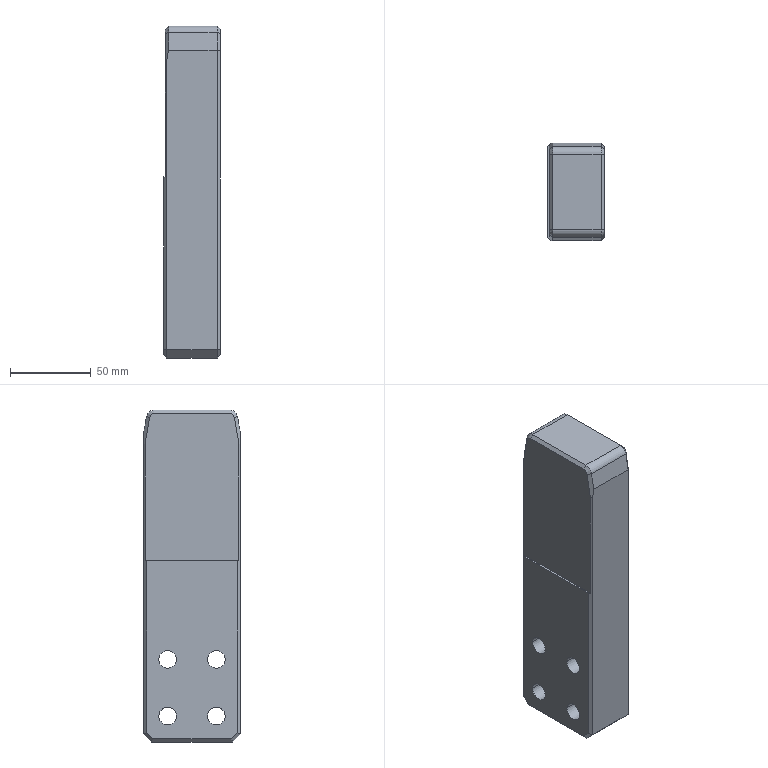Part | Creo | 1 solid | 54 faces | box 35 x 60 x 205 mm | volume 400314 mm3 | plane 32 | cylinder 18 | cone 4 | commonest cylinder face diameters 11 x8 18 x8 10 x2
STEP:
#1=CARTESIAN_POINT('',(299.5,-28.005,-15.));
#2=VERTEX_POINT('',#1);
#3=CARTESIAN_POINT('',(299.5,27.995,-15.));
#4=VERTEX_POINT('',#3);
#5=CARTESIAN_POINT('',(299.5,-28.005,-15.));
#6=DIRECTION('',(0.,1.,0.));
#7=VECTOR('',#6,56.);
#8=LINE('',#5,#7);
#9=EDGE_CURVE('',#2,#4,#8,.T.);
#10=ORIENTED_EDGE('',*,*,#9,.F.);
#11=CARTESIAN_POINT('',(299.5,-28.005,-121.172));
#12=VERTEX_POINT('',#11);
#13=CARTESIAN_POINT('',(299.5,-28.005,-15.));
#14=DIRECTION('',(0.,0.,-1.));
#15=VECTOR('',#14,106.172);
#16=LINE('',#13,#15);
#17=EDGE_CURVE('',#2,#12,#16,.T.);
#18=ORIENTED_EDGE('',*,*,#17,.T.);
#19=CARTESIAN_POINT('',(299.5,-24.176,-125.));
#20=VERTEX_POINT('',#19);
#21=CARTESIAN_POINT('',(299.5,-24.176,-125.));
#22=DIRECTION('',(0.,-0.7071,0.7071));
#23=VECTOR('',#22,5.414);
#24=LINE('',#21,#23);
#25=EDGE_CURVE('',#20,#12,#24,.T.);
#26=ORIENTED_EDGE('',*,*,#25,.F.);
#27=CARTESIAN_POINT('',(299.5,24.167,-125.));
#28=VERTEX_POINT('',#27);
#29=CARTESIAN_POINT('',(299.5,-24.176,-125.));
#30=DIRECTION('',(0.,1.,0.));
#31=VECTOR('',#30,48.343);
#32=LINE('',#29,#31);
#33=EDGE_CURVE('',#20,#28,#32,.T.);
#34=ORIENTED_EDGE('',*,*,#33,.T.);
#35=CARTESIAN_POINT('',(299.5,27.995,-121.172));
#36=VERTEX_POINT('',#35);
#37=CARTESIAN_POINT('',(299.5,27.995,-121.172));
#38=DIRECTION('',(0.,-0.7071,-0.7071));
#39=VECTOR('',#38,5.414);
#40=LINE('',#37,#39);
#41=EDGE_CURVE('',#36,#28,#40,.T.);
#42=ORIENTED_EDGE('',*,*,#41,.F.);
#43=CARTESIAN_POINT('',(299.5,27.995,-121.172));
#44=DIRECTION('',(0.,0.,1.));
#45=VECTOR('',#44,106.172);
#46=LINE('',#43,#45);
#47=EDGE_CURVE('',#36,#4,#46,.T.);
#48=ORIENTED_EDGE('',*,*,#47,.T.);
#49=EDGE_LOOP('',(#10,#18,#26,#34,#42,#48));
#50=FACE_OUTER_BOUND('',#49,.F.);
#51=CARTESIAN_POINT('',(299.5,-9.505,-76.));
#52=VERTEX_POINT('',#51);
#53=CARTESIAN_POINT('',(299.5,-20.505,-76.));
#54=VERTEX_POINT('',#53);
#55=CARTESIAN_POINT('',(299.5,-15.005,-76.));
#56=DIRECTION('',(1.,0.,0.));
#57=DIRECTION('',(0.,1.,0.));
#58=AXIS2_PLACEMENT_3D('',#55,#56,#57);
#59=CIRCLE('',#58,5.5);
#60=EDGE_CURVE('',#52,#54,#59,.T.);
#61=ORIENTED_EDGE('',*,*,#60,.F.);
#62=CARTESIAN_POINT('',(299.5,-15.005,-76.));
#63=DIRECTION('',(1.,0.,0.));
#64=DIRECTION('',(0.,-1.,0.));
#65=AXIS2_PLACEMENT_3D('',#62,#63,#64);
#66=CIRCLE('',#65,5.5);
#67=EDGE_CURVE('',#54,#52,#66,.T.);
#68=ORIENTED_EDGE('',*,*,#67,.F.);
#69=EDGE_LOOP('',(#61,#68));
#70=FACE_BOUND('',#69,.F.);
#71=CARTESIAN_POINT('',(299.5,20.495,-111.));
#72=VERTEX_POINT('',#71);
#73=CARTESIAN_POINT('',(299.5,9.495,-111.));
#74=VERTEX_POINT('',#73);
#75=CARTESIAN_POINT('',(299.5,14.995,-111.));
#76=DIRECTION('',(1.,0.,0.));
#77=DIRECTION('',(0.,1.,0.));
#78=AXIS2_PLACEMENT_3D('',#75,#76,#77);
#79=CIRCLE('',#78,5.5);
#80=EDGE_CURVE('',#72,#74,#79,.T.);
#81=ORIENTED_EDGE('',*,*,#80,.F.);
#82=CARTESIAN_POINT('',(299.5,14.995,-111.));
#83=DIRECTION('',(1.,0.,0.));
#84=DIRECTION('',(0.,-1.,0.));
#85=AXIS2_PLACEMENT_3D('',#82,#83,#84);
#86=CIRCLE('',#85,5.5);
#87=EDGE_CURVE('',#74,#72,#86,.T.);
#88=ORIENTED_EDGE('',*,*,#87,.F.);
#89=EDGE_LOOP('',(#81,#88));
#90=FACE_BOUND('',#89,.F.);
#91=CARTESIAN_POINT('',(299.5,20.495,-76.));
#92=VERTEX_POINT('',#91);
#93=CARTESIAN_POINT('',(299.5,9.495,-76.));
#94=VERTEX_POINT('',#93);
#95=CARTESIAN_POINT('',(299.5,14.995,-76.));
#96=DIRECTION('',(1.,0.,0.));
#97=DIRECTION('',(0.,1.,0.));
#98=AXIS2_PLACEMENT_3D('',#95,#96,#97);
#99=CIRCLE('',#98,5.5);
#100=EDGE_CURVE('',#92,#94,#99,.T.);
#101=ORIENTED_EDGE('',*,*,#100,.F.);
#102=CARTESIAN_POINT('',(299.5,14.995,-76.));
#103=DIRECTION('',(1.,0.,0.));
#104=DIRECTION('',(0.,-1.,0.));
#105=AXIS2_PLACEMENT_3D('',#102,#103,#104);
#106=CIRCLE('',#105,5.5);
#107=EDGE_CURVE('',#94,#92,#106,.T.);
#108=ORIENTED_EDGE('',*,*,#107,.F.);
#109=EDGE_LOOP('',(#101,#108));
#110=FACE_BOUND('',#109,.F.);
#111=CARTESIAN_POINT('',(299.5,-9.505,-111.));
#112=VERTEX_POINT('',#111);
#113=CARTESIAN_POINT('',(299.5,-20.505,-111.));
#114=VERTEX_POINT('',#113);
#115=CARTESIAN_POINT('',(299.5,-15.005,-111.));
#116=DIRECTION('',(1.,0.,0.));
#117=DIRECTION('',(0.,1.,0.));
#118=AXIS2_PLACEMENT_3D('',#115,#116,#117);
#119=CIRCLE('',#118,5.5);
#120=EDGE_CURVE('',#112,#114,#119,.T.);
#121=ORIENTED_EDGE('',*,*,#120,.F.);
#122=CARTESIAN_POINT('',(299.5,-15.005,-111.));
#123=DIRECTION('',(1.,0.,0.));
#124=DIRECTION('',(0.,-1.,0.));
#125=AXIS2_PLACEMENT_3D('',#122,#123,#124);
#126=CIRCLE('',#125,5.5);
#127=EDGE_CURVE('',#114,#112,#126,.T.);
#128=ORIENTED_EDGE('',*,*,#127,.F.);
#129=EDGE_LOOP('',(#121,#128));
#130=FACE_BOUND('',#129,.F.);
#131=CARTESIAN_POINT('',(299.5,-5.005,-87.));
#132=DIRECTION('',(-1.,0.,0.));
#133=DIRECTION('',(0.,0.,-1.));
#134=AXIS2_PLACEMENT_3D('',#131,#132,#133);
#135=PLANE('',#134);
#136=ADVANCED_FACE('',(#50,#70,#90,#110,#130),#135,.T.);
#137=CARTESIAN_POINT('',(323.5,9.495,-111.));
#138=VERTEX_POINT('',#137);
#139=CARTESIAN_POINT('',(323.5,14.995,-105.5));
#140=VERTEX_POINT('',#139);
#141=CARTESIAN_POINT('',(323.5,14.995,-111.));
#142=DIRECTION('',(-1.,0.,0.));
#143=DIRECTION('',(0.,-1.,0.));
#144=AXIS2_PLACEMENT_3D('',#141,#142,#143);
#145=CIRCLE('',#144,5.5);
#146=EDGE_CURVE('',#138,#140,#145,.T.);
#147=ORIENTED_EDGE('',*,*,#146,.T.);
#148=CARTESIAN_POINT('',(323.5,20.495,-111.));
#149=VERTEX_POINT('',#148);
#150=CARTESIAN_POINT('',(323.5,14.995,-111.));
#151=DIRECTION('',(-1.,0.,0.));
#152=DIRECTION('',(0.,0.,1.));
#153=AXIS2_PLACEMENT_3D('',#150,#151,#152);
#154=CIRCLE('',#153,5.5);
#155=EDGE_CURVE('',#140,#149,#154,.T.);
#156=ORIENTED_EDGE('',*,*,#155,.T.);
#157=CARTESIAN_POINT('',(323.5,20.495,-111.));
#158=DIRECTION('',(-1.,0.,0.));
#159=VECTOR('',#158,24.);
#160=LINE('',#157,#159);
#161=EDGE_CURVE('',#149,#72,#160,.T.);
#162=ORIENTED_EDGE('',*,*,#161,.T.);
#163=ORIENTED_EDGE('',*,*,#80,.T.);
#164=CARTESIAN_POINT('',(323.5,9.495,-111.));
#165=DIRECTION('',(-1.,0.,0.));
#166=VECTOR('',#165,24.);
#167=LINE('',#164,#166);
#168=EDGE_CURVE('',#138,#74,#167,.T.);
#169=ORIENTED_EDGE('',*,*,#168,.F.);
#170=EDGE_LOOP('',(#147,#156,#162,#163,#169));
#171=FACE_OUTER_BOUND('',#170,.F.);
#172=CARTESIAN_POINT('',(334.5,14.995,-111.));
#173=DIRECTION('',(-1.,0.,0.));
#174=DIRECTION('',(0.,1.,0.));
#175=AXIS2_PLACEMENT_3D('',#172,#173,#174);
#176=CYLINDRICAL_SURFACE('',#175,5.5);
#177=ADVANCED_FACE('',(#171),#176,.F.);
#178=CARTESIAN_POINT('',(323.5,23.995,-111.));
#179=VERTEX_POINT('',#178);
#180=CARTESIAN_POINT('',(323.5,5.995,-111.));
#181=VERTEX_POINT('',#180);
#182=CARTESIAN_POINT('',(323.5,14.995,-111.));
#183=DIRECTION('',(1.,0.,0.));
#184=DIRECTION('',(0.,1.,0.));
#185=AXIS2_PLACEMENT_3D('',#182,#183,#184);
#186=CIRCLE('',#185,9.);
#187=EDGE_CURVE('',#179,#181,#186,.T.);
#188=ORIENTED_EDGE('',*,*,#187,.F.);
#189=CARTESIAN_POINT('',(323.5,14.995,-111.));
#190=DIRECTION('',(1.,0.,0.));
#191=DIRECTION('',(0.,-1.,0.));
#192=AXIS2_PLACEMENT_3D('',#189,#190,#191);
#193=CIRCLE('',#192,9.);
#194=EDGE_CURVE('',#181,#179,#193,.T.);
#195=ORIENTED_EDGE('',*,*,#194,.F.);
#196=EDGE_LOOP('',(#188,#195));
#197=FACE_OUTER_BOUND('',#196,.F.);
#198=ORIENTED_EDGE('',*,*,#155,.F.);
#199=ORIENTED_EDGE('',*,*,#146,.F.);
#200=CARTESIAN_POINT('',(323.5,14.995,-111.));
#201=DIRECTION('',(-1.,0.,0.));
#202=DIRECTION('',(0.,1.,0.));
#203=AXIS2_PLACEMENT_3D('',#200,#201,#202);
#204=CIRCLE('',#203,5.5);
#205=EDGE_CURVE('',#149,#138,#204,.T.);
#206=ORIENTED_EDGE('',*,*,#205,.F.);
#207=EDGE_LOOP('',(#198,#199,#206));
#208=FACE_BOUND('',#207,.F.);
#209=CARTESIAN_POINT('',(323.5,14.995,-111.));
#210=DIRECTION('',(-1.,0.,0.));
#211=DIRECTION('',(0.,0.,1.));
#212=AXIS2_PLACEMENT_3D('',#209,#210,#211);
#213=PLANE('',#212);
#214=ADVANCED_FACE('',(#197,#208),#213,.F.);
#215=ORIENTED_EDGE('',*,*,#205,.T.);
#216=ORIENTED_EDGE('',*,*,#168,.T.);
#217=ORIENTED_EDGE('',*,*,#87,.T.);
#218=ORIENTED_EDGE('',*,*,#161,.F.);
#219=EDGE_LOOP('',(#215,#216,#217,#218));
#220=FACE_OUTER_BOUND('',#219,.F.);
#221=CARTESIAN_POINT('',(334.5,14.995,-111.));
#222=DIRECTION('',(-1.,0.,0.));
#223=DIRECTION('',(0.,1.,0.));
#224=AXIS2_PLACEMENT_3D('',#221,#222,#223);
#225=CYLINDRICAL_SURFACE('',#224,5.5);
#226=ADVANCED_FACE('',(#220),#225,.F.);
#227=ORIENTED_EDGE('',*,*,#187,.T.);
#228=CARTESIAN_POINT('',(334.5,5.995,-111.));
#229=VERTEX_POINT('',#228);
#230=CARTESIAN_POINT('',(334.5,5.995,-111.));
#231=DIRECTION('',(-1.,0.,0.));
#232=VECTOR('',#231,11.);
#233=LINE('',#230,#232);
#234=EDGE_CURVE('',#229,#181,#233,.T.);
#235=ORIENTED_EDGE('',*,*,#234,.F.);
#236=CARTESIAN_POINT('',(334.5,23.995,-111.));
#237=VERTEX_POINT('',#236);
#238=CARTESIAN_POINT('',(334.5,14.995,-111.));
#239=DIRECTION('',(-1.,0.,0.));
#240=DIRECTION('',(0.,-1.,0.));
#241=AXIS2_PLACEMENT_3D('',#238,#239,#240);
#242=CIRCLE('',#241,9.);
#243=EDGE_CURVE('',#229,#237,#242,.T.);
#244=ORIENTED_EDGE('',*,*,#243,.T.);
#245=CARTESIAN_POINT('',(334.5,23.995,-111.));
#246=DIRECTION('',(-1.,0.,0.));
#247=VECTOR('',#246,11.);
#248=LINE('',#245,#247);
#249=EDGE_CURVE('',#237,#179,#248,.T.);
#250=ORIENTED_EDGE('',*,*,#249,.T.);
#251=EDGE_LOOP('',(#227,#235,#244,#250));
#252=FACE_OUTER_BOUND('',#251,.F.);
#253=CARTESIAN_POINT('',(334.5,14.995,-111.));
#254=DIRECTION('',(-1.,0.,0.));
#255=DIRECTION('',(0.,1.,0.));
#256=AXIS2_PLACEMENT_3D('',#253,#254,#255);
#257=CYLINDRICAL_SURFACE('',#256,9.);
#258=ADVANCED_FACE('',(#252),#257,.F.);
#259=ORIENTED_EDGE('',*,*,#194,.T.);
#260=ORIENTED_EDGE('',*,*,#249,.F.);
#261=CARTESIAN_POINT('',(334.5,14.995,-111.));
#262=DIRECTION('',(-1.,0.,0.));
#263=DIRECTION('',(0.,1.,0.));
#264=AXIS2_PLACEMENT_3D('',#261,#262,#263);
#265=CIRCLE('',#264,9.);
#266=EDGE_CURVE('',#237,#229,#265,.T.);
#267=ORIENTED_EDGE('',*,*,#266,.T.);
#268=ORIENTED_EDGE('',*,*,#234,.T.);
#269=EDGE_LOOP('',(#259,#260,#267,#268));
#270=FACE_OUTER_BOUND('',#269,.F.);
#271=CARTESIAN_POINT('',(334.5,14.995,-111.));
#272=DIRECTION('',(-1.,0.,0.));
#273=DIRECTION('',(0.,1.,0.));
#274=AXIS2_PLACEMENT_3D('',#271,#272,#273);
#275=CYLINDRICAL_SURFACE('',#274,9.);
#276=ADVANCED_FACE('',(#270),#275,.F.);
#277=CARTESIAN_POINT('',(334.5,24.167,-125.));
#278=VERTEX_POINT('',#277);
#279=CARTESIAN_POINT('',(334.5,-24.176,-125.));
#280=VERTEX_POINT('',#279);
#281=CARTESIAN_POINT('',(334.5,24.167,-125.));
#282=DIRECTION('',(0.,-1.,0.));
#283=VECTOR('',#282,48.343);
#284=LINE('',#281,#283);
#285=EDGE_CURVE('',#278,#280,#284,.T.);
#286=ORIENTED_EDGE('',*,*,#285,.T.);
#287=CARTESIAN_POINT('',(334.5,-28.005,-121.172));
#288=VERTEX_POINT('',#287);
#289=CARTESIAN_POINT('',(334.5,-28.005,-121.172));
#290=DIRECTION('',(0.,0.7071,-0.7071));
#291=VECTOR('',#290,5.414);
#292=LINE('',#289,#291);
#293=EDGE_CURVE('',#288,#280,#292,.T.);
#294=ORIENTED_EDGE('',*,*,#293,.F.);
#295=CARTESIAN_POINT('',(334.5,-28.005,62.825));
#296=VERTEX_POINT('',#295);
#297=CARTESIAN_POINT('',(334.5,-28.005,-121.172));
#298=DIRECTION('',(0.,0.,1.));
#299=VECTOR('',#298,183.997);
#300=LINE('',#297,#299);
#301=EDGE_CURVE('',#288,#296,#300,.T.);
#302=ORIENTED_EDGE('',*,*,#301,.T.);
#303=CARTESIAN_POINT('',(334.5,-26.119,73.521));
#304=VERTEX_POINT('',#303);
#305=CARTESIAN_POINT('',(334.5,-26.119,73.521));
#306=DIRECTION('',(0.,-0.1736,-0.9848));
#307=VECTOR('',#306,10.861);
#308=LINE('',#305,#307);
#309=EDGE_CURVE('',#304,#296,#308,.T.);
#310=ORIENTED_EDGE('',*,*,#309,.F.);
#311=CARTESIAN_POINT('',(334.5,-23.164,76.));
#312=VERTEX_POINT('',#311);
#313=CARTESIAN_POINT('',(334.5,-23.164,73.));
#314=DIRECTION('',(1.,0.,0.));
#315=DIRECTION('',(0.,0.,1.));
#316=AXIS2_PLACEMENT_3D('',#313,#314,#315);
#317=CIRCLE('',#316,3.);
#318=EDGE_CURVE('',#312,#304,#317,.T.);
#319=ORIENTED_EDGE('',*,*,#318,.F.);
#320=CARTESIAN_POINT('',(334.5,23.155,76.));
#321=VERTEX_POINT('',#320);
#322=CARTESIAN_POINT('',(334.5,-23.164,76.));
#323=DIRECTION('',(0.,1.,0.));
#324=VECTOR('',#323,46.319);
#325=LINE('',#322,#324);
#326=EDGE_CURVE('',#312,#321,#325,.T.);
#327=ORIENTED_EDGE('',*,*,#326,.T.);
#328=CARTESIAN_POINT('',(334.5,26.109,73.521));
#329=VERTEX_POINT('',#328);
#330=CARTESIAN_POINT('',(334.5,23.155,73.));
#331=DIRECTION('',(1.,0.,0.));
#332=DIRECTION('',(0.,0.9848,0.1736));
#333=AXIS2_PLACEMENT_3D('',#330,#331,#332);
#334=CIRCLE('',#333,3.);
#335=EDGE_CURVE('',#329,#321,#334,.T.);
#336=ORIENTED_EDGE('',*,*,#335,.F.);
#337=CARTESIAN_POINT('',(334.5,27.995,62.825));
#338=VERTEX_POINT('',#337);
#339=CARTESIAN_POINT('',(334.5,27.995,62.825));
#340=DIRECTION('',(0.,-0.1736,0.9848));
#341=VECTOR('',#340,10.861);
#342=LINE('',#339,#341);
#343=EDGE_CURVE('',#338,#329,#342,.T.);
#344=ORIENTED_EDGE('',*,*,#343,.F.);
#345=CARTESIAN_POINT('',(334.5,27.995,-121.172));
#346=VERTEX_POINT('',#345);
#347=CARTESIAN_POINT('',(334.5,27.995,62.825));
#348=DIRECTION('',(0.,0.,-1.));
#349=VECTOR('',#348,183.997);
#350=LINE('',#347,#349);
#351=EDGE_CURVE('',#338,#346,#350,.T.);
#352=ORIENTED_EDGE('',*,*,#351,.T.);
#353=CARTESIAN_POINT('',(334.5,24.167,-125.));
#354=DIRECTION('',(0.,0.7071,0.7071));
#355=VECTOR('',#354,5.414);
#356=LINE('',#353,#355);
#357=EDGE_CURVE('',#278,#346,#356,.T.);
#358=ORIENTED_EDGE('',*,*,#357,.F.);
#359=EDGE_LOOP('',(#286,#294,#302,#310,#319,#327,#336,#344,#352,#358));
#360=FACE_OUTER_BOUND('',#359,.F.);
#361=ORIENTED_EDGE('',*,*,#266,.F.);
#362=ORIENTED_EDGE('',*,*,#243,.F.);
#363=EDGE_LOOP('',(#361,#362));
#364=FACE_BOUND('',#363,.F.);
#365=CARTESIAN_POINT('',(334.5,-6.005,-76.));
#366=VERTEX_POINT('',#365);
#367=CARTESIAN_POINT('',(334.5,-24.005,-76.));
#368=VERTEX_POINT('',#367);
#369=CARTESIAN_POINT('',(334.5,-15.005,-76.));
#370=DIRECTION('',(-1.,0.,0.));
#371=DIRECTION('',(0.,1.,0.));
#372=AXIS2_PLACEMENT_3D('',#369,#370,#371);
#373=CIRCLE('',#372,9.);
#374=EDGE_CURVE('',#366,#368,#373,.T.);
#375=ORIENTED_EDGE('',*,*,#374,.F.);
#376=CARTESIAN_POINT('',(334.5,-15.005,-76.));
#377=DIRECTION('',(-1.,0.,0.));
#378=DIRECTION('',(0.,-1.,0.));
#379=AXIS2_PLACEMENT_3D('',#376,#377,#378);
#380=CIRCLE('',#379,9.);
#381=EDGE_CURVE('',#368,#366,#380,.T.);
#382=ORIENTED_EDGE('',*,*,#381,.F.);
#383=EDGE_LOOP('',(#375,#382));
#384=FACE_BOUND('',#383,.F.);
#385=CARTESIAN_POINT('',(334.5,23.995,-76.));
#386=VERTEX_POINT('',#385);
#387=CARTESIAN_POINT('',(334.5,5.995,-76.));
#388=VERTEX_POINT('',#387);
#389=CARTESIAN_POINT('',(334.5,14.995,-76.));
#390=DIRECTION('',(-1.,0.,0.));
#391=DIRECTION('',(0.,1.,0.));
#392=AXIS2_PLACEMENT_3D('',#389,#390,#391);
#393=CIRCLE('',#392,9.);
#394=EDGE_CURVE('',#386,#388,#393,.T.);
#395=ORIENTED_EDGE('',*,*,#394,.F.);
#396=CARTESIAN_POINT('',(334.5,14.995,-76.));
#397=DIRECTION('',(-1.,0.,0.));
#398=DIRECTION('',(0.,-1.,0.));
#399=AXIS2_PLACEMENT_3D('',#396,#397,#398);
#400=CIRCLE('',#399,9.);
#401=EDGE_CURVE('',#388,#386,#400,.T.);
#402=ORIENTED_EDGE('',*,*,#401,.F.);
#403=EDGE_LOOP('',(#395,#402));
#404=FACE_BOUND('',#403,.F.);
#405=CARTESIAN_POINT('',(334.5,-6.005,-111.));
#406=VERTEX_POINT('',#405);
#407=CARTESIAN_POINT('',(334.5,-24.005,-111.));
#408=VERTEX_POINT('',#407);
#409=CARTESIAN_POINT('',(334.5,-15.005,-111.));
#410=DIRECTION('',(-1.,0.,0.));
#411=DIRECTION('',(0.,1.,0.));
#412=AXIS2_PLACEMENT_3D('',#409,#410,#411);
#413=CIRCLE('',#412,9.);
#414=EDGE_CURVE('',#406,#408,#413,.T.);
#415=ORIENTED_EDGE('',*,*,#414,.F.);
#416=CARTESIAN_POINT('',(334.5,-15.005,-111.));
#417=DIRECTION('',(-1.,0.,0.));
#418=DIRECTION('',(0.,-1.,0.));
#419=AXIS2_PLACEMENT_3D('',#416,#417,#418);
#420=CIRCLE('',#419,9.);
#421=EDGE_CURVE('',#408,#406,#420,.T.);
#422=ORIENTED_EDGE('',*,*,#421,.F.);
#423=EDGE_LOOP('',(#415,#422));
#424=FACE_BOUND('',#423,.F.);
#425=CARTESIAN_POINT('',(334.5,-5.005,-87.));
#426=DIRECTION('',(1.,0.,0.));
#427=DIRECTION('',(0.,0.,1.));
#428=AXIS2_PLACEMENT_3D('',#425,#426,#427);
#429=PLANE('',#428);
#430=ADVANCED_FACE('',(#360,#364,#384,#404,#424),#429,.T.);
#431=CARTESIAN_POINT('',(332.5,-25.005,-127.));
#432=VERTEX_POINT('',#431);
#433=CARTESIAN_POINT('',(332.5,-25.005,-127.));
#434=DIRECTION('',(0.6786,0.2811,0.6786));
#435=VECTOR('',#434,2.947);
#436=LINE('',#433,#435);
#437=EDGE_CURVE('',#432,#280,#436,.T.);
#438=ORIENTED_EDGE('',*,*,#437,.T.);
#439=ORIENTED_EDGE('',*,*,#285,.F.);
#440=CARTESIAN_POINT('',(332.5,24.995,-127.));
#441=VERTEX_POINT('',#440);
#442=CARTESIAN_POINT('',(332.5,24.995,-127.));
#443=DIRECTION('',(0.6786,-0.2811,0.6786));
#444=VECTOR('',#443,2.947);
#445=LINE('',#442,#444);
#446=EDGE_CURVE('',#441,#278,#445,.T.);
#447=ORIENTED_EDGE('',*,*,#446,.F.);
#448=CARTESIAN_POINT('',(332.5,-25.005,-127.));
#449=DIRECTION('',(0.,1.,0.));
#450=VECTOR('',#449,50.);
#451=LINE('',#448,#450);
#452=EDGE_CURVE('',#432,#441,#451,.T.);
#453=ORIENTED_EDGE('',*,*,#452,.F.);
#454=EDGE_LOOP('',(#438,#439,#447,#453));
#455=FACE_OUTER_BOUND('',#454,.F.);
#456=CARTESIAN_POINT('',(334.5,-5.005,-125.));
#457=DIRECTION('',(-0.7071,0.,0.7071));
#458=DIRECTION('',(0.,1.,0.));
#459=AXIS2_PLACEMENT_3D('',#456,#457,#458);
#460=PLANE('',#459);
#461=ADVANCED_FACE('',(#455),#460,.F.);
#462=CARTESIAN_POINT('',(332.5,-30.005,-122.));
#463=VERTEX_POINT('',#462);
#464=CARTESIAN_POINT('',(332.5,-30.005,-122.));
#465=DIRECTION('',(0.6786,0.6786,0.2811));
#466=VECTOR('',#465,2.947);
#467=LINE('',#464,#466);
#468=EDGE_CURVE('',#463,#288,#467,.T.);
#469=ORIENTED_EDGE('',*,*,#468,.T.);
#470=ORIENTED_EDGE('',*,*,#293,.T.);
#471=ORIENTED_EDGE('',*,*,#437,.F.);
#472=CARTESIAN_POINT('',(332.5,-30.005,-122.));
#473=DIRECTION('',(0.,0.7071,-0.7071));
#474=VECTOR('',#473,7.071);
#475=LINE('',#472,#474);
#476=EDGE_CURVE('',#463,#432,#475,.T.);
#477=ORIENTED_EDGE('',*,*,#476,.F.);
#478=EDGE_LOOP('',(#469,#470,#471,#477));
#479=FACE_OUTER_BOUND('',#478,.F.);
#480=CARTESIAN_POINT('',(334.5,-33.59,-115.586));
#481=DIRECTION('',(0.7071,-0.5,-0.5));
#482=DIRECTION('',(0.,-0.7071,0.7071));
#483=AXIS2_PLACEMENT_3D('',#480,#481,#482);
#484=PLANE('',#483);
#485=ADVANCED_FACE('',(#479),#484,.T.);
#486=CARTESIAN_POINT('',(332.5,-30.005,63.));
#487=VERTEX_POINT('',#486);
#488=CARTESIAN_POINT('',(332.5,-30.005,63.));
#489=DIRECTION('',(0.7058,0.7058,-0.06175));
#490=VECTOR('',#489,2.834);
#491=LINE('',#488,#490);
#492=EDGE_CURVE('',#487,#296,#491,.T.);
#493=ORIENTED_EDGE('',*,*,#492,.T.);
#494=ORIENTED_EDGE('',*,*,#301,.F.);
#495=ORIENTED_EDGE('',*,*,#468,.F.);
#496=CARTESIAN_POINT('',(332.5,-30.005,63.));
#497=DIRECTION('',(0.,0.,-1.));
#498=VECTOR('',#497,185.);
#499=LINE('',#496,#498);
#500=EDGE_CURVE('',#487,#463,#499,.T.);
#501=ORIENTED_EDGE('',*,*,#500,.F.);
#502=EDGE_LOOP('',(#493,#494,#495,#501));
#503=FACE_OUTER_BOUND('',#502,.F.);
#504=CARTESIAN_POINT('',(332.5,-30.005,-87.));
#505=DIRECTION('',(-0.7071,0.7071,0.));
#506=DIRECTION('',(0.,0.,1.));
#507=AXIS2_PLACEMENT_3D('',#504,#505,#506);
#508=PLANE('',#507);
#509=ADVANCED_FACE('',(#503),#508,.F.);
#510=CARTESIAN_POINT('',(332.5,-28.088,73.868));
#511=VERTEX_POINT('',#510);
#512=CARTESIAN_POINT('',(332.5,-28.088,73.868));
#513=DIRECTION('',(0.7071,0.6964,-0.1228));
#514=VECTOR('',#513,2.828);
#515=LINE('',#512,#514);
#516=EDGE_CURVE('',#511,#304,#515,.T.);
#517=ORIENTED_EDGE('',*,*,#516,.T.);
#518=ORIENTED_EDGE('',*,*,#309,.T.);
#519=ORIENTED_EDGE('',*,*,#492,.F.);
#520=CARTESIAN_POINT('',(332.5,-28.088,73.868));
#521=DIRECTION('',(0.,-0.1736,-0.9848));
#522=VECTOR('',#521,11.036);
#523=LINE('',#520,#522);
#524=EDGE_CURVE('',#511,#487,#523,.T.);
#525=ORIENTED_EDGE('',*,*,#524,.F.);
#526=EDGE_LOOP('',(#517,#518,#519,#525));
#527=FACE_OUTER_BOUND('',#526,.F.);
#528=CARTESIAN_POINT('',(332.5,-30.005,63.));
#529=DIRECTION('',(-0.7071,0.6964,-0.1228));
#530=DIRECTION('',(0.,0.1736,0.9848));
#531=AXIS2_PLACEMENT_3D('',#528,#529,#530);
#532=PLANE('',#531);
#533=ADVANCED_FACE('',(#527),#532,.F.);
#534=CARTESIAN_POINT('',(332.5,-23.164,78.));
#535=VERTEX_POINT('',#534);
#536=CARTESIAN_POINT('',(334.5,-23.164,76.));
#537=DIRECTION('',(-0.7071,0.,0.7071));
#538=VECTOR('',#537,2.828);
#539=LINE('',#536,#538);
#540=EDGE_CURVE('',#312,#535,#539,.T.);
#541=ORIENTED_EDGE('',*,*,#540,.F.);
#542=ORIENTED_EDGE('',*,*,#318,.T.);
#543=ORIENTED_EDGE('',*,*,#516,.F.);
#544=CARTESIAN_POINT('',(332.5,-23.164,73.));
#545=DIRECTION('',(1.,0.,0.));
#546=DIRECTION('',(0.,0.,1.));
#547=AXIS2_PLACEMENT_3D('',#544,#545,#546);
#548=CIRCLE('',#547,5.);
#549=EDGE_CURVE('',#535,#511,#548,.T.);
#550=ORIENTED_EDGE('',*,*,#549,.F.);
#551=EDGE_LOOP('',(#541,#542,#543,#550));
#552=FACE_OUTER_BOUND('',#551,.F.);
#553=CARTESIAN_POINT('',(333.5,-23.164,73.));
#554=DIRECTION('',(-1.,0.,0.));
#555=DIRECTION('',(0.,0.,-1.));
#556=AXIS2_PLACEMENT_3D('',#553,#554,#555);
#557=CONICAL_SURFACE('',#556,4.,45.);
#558=ADVANCED_FACE('',(#552),#557,.T.);
#559=ORIENTED_EDGE('',*,*,#540,.T.);
#560=CARTESIAN_POINT('',(332.5,23.155,78.));
#561=VERTEX_POINT('',#560);
#562=CARTESIAN_POINT('',(332.5,23.155,78.));
#563=DIRECTION('',(0.,-1.,0.));
#564=VECTOR('',#563,46.319);
#565=LINE('',#562,#564);
#566=EDGE_CURVE('',#561,#535,#565,.T.);
#567=ORIENTED_EDGE('',*,*,#566,.F.);
#568=CARTESIAN_POINT('',(332.5,23.155,78.));
#569=DIRECTION('',(0.7071,0.,-0.7071));
#570=VECTOR('',#569,2.828);
#571=LINE('',#568,#570);
#572=EDGE_CURVE('',#561,#321,#571,.T.);
#573=ORIENTED_EDGE('',*,*,#572,.T.);
#574=ORIENTED_EDGE('',*,*,#326,.F.);
#575=EDGE_LOOP('',(#559,#567,#573,#574));
#576=FACE_OUTER_BOUND('',#575,.F.);
#577=CARTESIAN_POINT('',(334.5,-5.005,76.));
#578=DIRECTION('',(0.7071,0.,0.7071));
#579=DIRECTION('',(0.,1.,0.));
#580=AXIS2_PLACEMENT_3D('',#577,#578,#579);
#581=PLANE('',#580);
#582=ADVANCED_FACE('',(#576),#581,.T.);
#583=CARTESIAN_POINT('',(302.5,23.155,78.));
#584=VERTEX_POINT('',#583);
#585=CARTESIAN_POINT('',(302.5,23.155,78.));
#586=DIRECTION('',(1.,0.,0.));
#587=VECTOR('',#586,30.);
#588=LINE('',#585,#587);
#589=EDGE_CURVE('',#584,#561,#588,.T.);
#590=ORIENTED_EDGE('',*,*,#589,.T.);
#591=ORIENTED_EDGE('',*,*,#566,.T.);
#592=CARTESIAN_POINT('',(302.5,-23.164,78.));
#593=VERTEX_POINT('',#592);
#594=CARTESIAN_POINT('',(332.5,-23.164,78.));
#595=DIRECTION('',(-1.,0.,0.));
#596=VECTOR('',#595,30.);
#597=LINE('',#594,#596);
#598=EDGE_CURVE('',#535,#593,#597,.T.);
#599=ORIENTED_EDGE('',*,*,#598,.T.);
#600=CARTESIAN_POINT('',(302.5,-23.164,78.));
#601=DIRECTION('',(0.,1.,0.));
#602=VECTOR('',#601,46.319);
#603=LINE('',#600,#602);
#604=EDGE_CURVE('',#593,#584,#603,.T.);
#605=ORIENTED_EDGE('',*,*,#604,.T.);
#606=EDGE_LOOP('',(#590,#591,#599,#605));
#607=FACE_OUTER_BOUND('',#606,.F.);
#608=CARTESIAN_POINT('',(318.5,42.745,78.));
#609=DIRECTION('',(0.,0.,-1.));
#610=DIRECTION('',(1.,0.,0.));
#611=AXIS2_PLACEMENT_3D('',#608,#609,#610);
#612=PLANE('',#611);
#613=ADVANCED_FACE('',(#607),#612,.F.);
#614=CARTESIAN_POINT('',(332.5,28.079,73.868));
#615=VERTEX_POINT('',#614);
#616=CARTESIAN_POINT('',(302.5,28.079,73.868));
#617=VERTEX_POINT('',#616);
#618=CARTESIAN_POINT('',(332.5,28.079,73.868));
#619=DIRECTION('',(-1.,0.,0.));
#620=VECTOR('',#619,30.);
#621=LINE('',#618,#620);
#622=EDGE_CURVE('',#615,#617,#621,.T.);
#623=ORIENTED_EDGE('',*,*,#622,.F.);
#624=CARTESIAN_POINT('',(332.5,23.155,73.));
#625=DIRECTION('',(1.,0.,0.));
#626=DIRECTION('',(0.,0.9848,0.1736));
#627=AXIS2_PLACEMENT_3D('',#624,#625,#626);
#628=CIRCLE('',#627,5.);
#629=EDGE_CURVE('',#615,#561,#628,.T.);
#630=ORIENTED_EDGE('',*,*,#629,.T.);
#631=ORIENTED_EDGE('',*,*,#589,.F.);
#632=CARTESIAN_POINT('',(302.5,23.155,73.));
#633=DIRECTION('',(-1.,0.,0.));
#634=DIRECTION('',(0.,0.,1.));
#635=AXIS2_PLACEMENT_3D('',#632,#633,#634);
#636=CIRCLE('',#635,5.);
#637=EDGE_CURVE('',#584,#617,#636,.T.);
#638=ORIENTED_EDGE('',*,*,#637,.T.);
#639=EDGE_LOOP('',(#623,#630,#631,#638));
#640=FACE_OUTER_BOUND('',#639,.F.);
#641=CARTESIAN_POINT('',(317.,23.155,73.));
#642=DIRECTION('',(-1.,0.,0.));
#643=DIRECTION('',(0.,0.,-1.));
#644=AXIS2_PLACEMENT_3D('',#641,#642,#643);
#645=CYLINDRICAL_SURFACE('',#644,5.);
#646=ADVANCED_FACE('',(#640),#645,.T.);
#647=CARTESIAN_POINT('',(302.5,29.995,63.));
#648=VERTEX_POINT('',#647);
#649=CARTESIAN_POINT('',(332.5,29.995,63.));
#650=VERTEX_POINT('',#649);
#651=CARTESIAN_POINT('',(302.5,29.995,63.));
#652=DIRECTION('',(1.,0.,0.));
#653=VECTOR('',#652,30.);
#654=LINE('',#651,#653);
#655=EDGE_CURVE('',#648,#650,#654,.T.);
#656=ORIENTED_EDGE('',*,*,#655,.T.);
#657=CARTESIAN_POINT('',(332.5,29.995,63.));
#658=DIRECTION('',(0.,-0.1736,0.9848));
#659=VECTOR('',#658,11.036);
#660=LINE('',#657,#659);
#661=EDGE_CURVE('',#650,#615,#660,.T.);
#662=ORIENTED_EDGE('',*,*,#661,.T.);
#663=ORIENTED_EDGE('',*,*,#622,.T.);
#664=CARTESIAN_POINT('',(302.5,28.079,73.868));
#665=DIRECTION('',(0.,0.1736,-0.9848));
#666=VECTOR('',#665,11.036);
#667=LINE('',#664,#666);
#668=EDGE_CURVE('',#617,#648,#667,.T.);
#669=ORIENTED_EDGE('',*,*,#668,.T.);
#670=EDGE_LOOP('',(#656,#662,#663,#669));
#671=FACE_OUTER_BOUND('',#670,.F.);
#672=CARTESIAN_POINT('',(317.,29.995,63.));
#673=DIRECTION('',(0.,0.9848,0.1736));
#674=DIRECTION('',(0.,0.1736,-0.9848));
#675=AXIS2_PLACEMENT_3D('',#672,#673,#674);
#676=PLANE('',#675);
#677=ADVANCED_FACE('',(#671),#676,.T.);
#678=CARTESIAN_POINT('',(301.5,29.995,57.241));
#679=VERTEX_POINT('',#678);
#680=CARTESIAN_POINT('',(301.5,29.995,-122.));
#681=VERTEX_POINT('',#680);
#682=CARTESIAN_POINT('',(301.5,29.995,57.241));
#683=DIRECTION('',(0.,0.,-1.));
#684=VECTOR('',#683,179.241);
#685=LINE('',#682,#684);
#686=EDGE_CURVE('',#679,#681,#685,.T.);
#687=ORIENTED_EDGE('',*,*,#686,.T.);
#688=CARTESIAN_POINT('',(332.5,29.995,-122.));
#689=VERTEX_POINT('',#688);
#690=CARTESIAN_POINT('',(301.5,29.995,-122.));
#691=DIRECTION('',(1.,0.,0.));
#692=VECTOR('',#691,31.);
#693=LINE('',#690,#692);
#694=EDGE_CURVE('',#681,#689,#693,.T.);
#695=ORIENTED_EDGE('',*,*,#694,.T.);
#696=CARTESIAN_POINT('',(332.5,29.995,-122.));
#697=DIRECTION('',(0.,0.,1.));
#698=VECTOR('',#697,185.);
#699=LINE('',#696,#698);
#700=EDGE_CURVE('',#689,#650,#699,.T.);
#701=ORIENTED_EDGE('',*,*,#700,.T.);
#702=ORIENTED_EDGE('',*,*,#655,.F.);
#703=CARTESIAN_POINT('',(302.5,29.995,63.));
#704=DIRECTION('',(-0.1711,0.,-0.9853));
#705=VECTOR('',#704,5.845);
#706=LINE('',#703,#705);
#707=EDGE_CURVE('',#648,#679,#706,.T.);
#708=ORIENTED_EDGE('',*,*,#707,.T.);
#709=EDGE_LOOP('',(#687,#695,#701,#702,#708));
#710=FACE_OUTER_BOUND('',#709,.F.);
#711=CARTESIAN_POINT('',(318.5,29.995,-87.));
#712=DIRECTION('',(0.,1.,0.));
#713=DIRECTION('',(0.,0.,-1.));
#714=AXIS2_PLACEMENT_3D('',#711,#712,#713);
#715=PLANE('',#714);
#716=ADVANCED_FACE('',(#710),#715,.T.);
#717=CARTESIAN_POINT('',(300.5,28.995,-15.));
#718=VERTEX_POINT('',#717);
#719=CARTESIAN_POINT('',(300.5,28.995,57.154));
#720=VERTEX_POINT('',#719);
#721=CARTESIAN_POINT('',(300.5,28.995,-15.));
#722=DIRECTION('',(0.,0.,1.));
#723=VECTOR('',#722,72.154);
#724=LINE('',#721,#723);
#725=EDGE_CURVE('',#718,#720,#724,.T.);
#726=ORIENTED_EDGE('',*,*,#725,.F.);
#727=CARTESIAN_POINT('',(300.5,28.995,-15.));
#728=DIRECTION('',(-0.7071,-0.7071,0.));
#729=VECTOR('',#728,1.414);
#730=LINE('',#727,#729);
#731=EDGE_CURVE('',#718,#4,#730,.T.);
#732=ORIENTED_EDGE('',*,*,#731,.T.);
#733=ORIENTED_EDGE('',*,*,#47,.F.);
#734=CARTESIAN_POINT('',(299.5,27.995,-121.172));
#735=DIRECTION('',(0.6786,0.6786,-0.2811));
#736=VECTOR('',#735,2.947);
#737=LINE('',#734,#736);
#738=EDGE_CURVE('',#36,#681,#737,.T.);
#739=ORIENTED_EDGE('',*,*,#738,.T.);
#740=ORIENTED_EDGE('',*,*,#686,.F.);
#741=CARTESIAN_POINT('',(301.5,29.995,57.241));
#742=DIRECTION('',(-0.7058,-0.7058,-0.06175));
#743=VECTOR('',#742,1.417);
#744=LINE('',#741,#743);
#745=EDGE_CURVE('',#679,#720,#744,.T.);
#746=ORIENTED_EDGE('',*,*,#745,.T.);
#747=EDGE_LOOP('',(#726,#732,#733,#739,#740,#746));
#748=FACE_OUTER_BOUND('',#747,.F.);
#749=CARTESIAN_POINT('',(301.5,29.995,-87.));
#750=DIRECTION('',(0.7071,-0.7071,0.));
#751=DIRECTION('',(0.,0.,1.));
#752=AXIS2_PLACEMENT_3D('',#749,#750,#751);
#753=PLANE('',#752);
#754=ADVANCED_FACE('',(#748),#753,.F.);
#755=CARTESIAN_POINT('',(300.5,23.155,76.));
#756=VERTEX_POINT('',#755);
#757=CARTESIAN_POINT('',(300.5,26.109,73.521));
#758=VERTEX_POINT('',#757);
#759=CARTESIAN_POINT('',(300.5,23.155,73.));
#760=DIRECTION('',(-1.,0.,0.));
#761=DIRECTION('',(0.,0.,1.));
#762=AXIS2_PLACEMENT_3D('',#759,#760,#761);
#763=CIRCLE('',#762,3.);
#764=EDGE_CURVE('',#756,#758,#763,.T.);
#765=ORIENTED_EDGE('',*,*,#764,.F.);
#766=CARTESIAN_POINT('',(300.5,-23.164,76.));
#767=VERTEX_POINT('',#766);
#768=CARTESIAN_POINT('',(300.5,23.155,76.));
#769=DIRECTION('',(0.,-1.,0.));
#770=VECTOR('',#769,46.319);
#771=LINE('',#768,#770);
#772=EDGE_CURVE('',#756,#767,#771,.T.);
#773=ORIENTED_EDGE('',*,*,#772,.T.);
#774=CARTESIAN_POINT('',(300.5,-26.119,73.521));
#775=VERTEX_POINT('',#774);
#776=CARTESIAN_POINT('',(300.5,-23.164,73.));
#777=DIRECTION('',(-1.,0.,0.));
#778=DIRECTION('',(0.,-0.9848,0.1736));
#779=AXIS2_PLACEMENT_3D('',#776,#777,#778);
#780=CIRCLE('',#779,3.);
#781=EDGE_CURVE('',#775,#767,#780,.T.);
#782=ORIENTED_EDGE('',*,*,#781,.F.);
#783=CARTESIAN_POINT('',(300.5,-29.005,57.154));
#784=VERTEX_POINT('',#783);
#785=CARTESIAN_POINT('',(300.5,-29.005,57.154));
#786=DIRECTION('',(0.,0.1736,0.9848));
#787=VECTOR('',#786,16.62);
#788=LINE('',#785,#787);
#789=EDGE_CURVE('',#784,#775,#788,.T.);
#790=ORIENTED_EDGE('',*,*,#789,.F.);
#791=CARTESIAN_POINT('',(300.5,-29.005,-15.));
#792=VERTEX_POINT('',#791);
#793=CARTESIAN_POINT('',(300.5,-29.005,57.154));
#794=DIRECTION('',(0.,0.,-1.));
#795=VECTOR('',#794,72.154);
#796=LINE('',#793,#795);
#797=EDGE_CURVE('',#784,#792,#796,.T.);
#798=ORIENTED_EDGE('',*,*,#797,.T.);
#799=CARTESIAN_POINT('',(300.5,-29.005,-15.));
#800=DIRECTION('',(0.,1.,0.));
#801=VECTOR('',#800,58.);
#802=LINE('',#799,#801);
#803=EDGE_CURVE('',#792,#718,#802,.T.);
#804=ORIENTED_EDGE('',*,*,#803,.T.);
#805=ORIENTED_EDGE('',*,*,#725,.T.);
#806=CARTESIAN_POINT('',(300.5,26.109,73.521));
#807=DIRECTION('',(0.,0.1736,-0.9848));
#808=VECTOR('',#807,16.62);
#809=LINE('',#806,#808);
#810=EDGE_CURVE('',#758,#720,#809,.T.);
#811=ORIENTED_EDGE('',*,*,#810,.F.);
#812=EDGE_LOOP('',(#765,#773,#782,#790,#798,#804,#805,#811));
#813=FACE_OUTER_BOUND('',#812,.F.);
#814=CARTESIAN_POINT('',(300.5,42.745,-10.));
#815=DIRECTION('',(-1.,0.,0.));
#816=DIRECTION('',(0.,0.,-1.));
#817=AXIS2_PLACEMENT_3D('',#814,#815,#816);
#818=PLANE('',#817);
#819=ADVANCED_FACE('',(#813),#818,.T.);
#820=CARTESIAN_POINT('',(300.5,23.155,76.));
#821=DIRECTION('',(0.7071,0.,0.7071));
#822=VECTOR('',#821,2.828);
#823=LINE('',#820,#822);
#824=EDGE_CURVE('',#756,#584,#823,.T.);
#825=ORIENTED_EDGE('',*,*,#824,.F.);
#826=ORIENTED_EDGE('',*,*,#764,.T.);
#827=CARTESIAN_POINT('',(302.5,28.079,73.868));
#828=DIRECTION('',(-0.7071,-0.6964,-0.1228));
#829=VECTOR('',#828,2.828);
#830=LINE('',#827,#829);
#831=EDGE_CURVE('',#617,#758,#830,.T.);
#832=ORIENTED_EDGE('',*,*,#831,.F.);
#833=ORIENTED_EDGE('',*,*,#637,.F.);
#834=EDGE_LOOP('',(#825,#826,#832,#833));
#835=FACE_OUTER_BOUND('',#834,.F.);
#836=CARTESIAN_POINT('',(301.5,23.155,73.));
#837=DIRECTION('',(1.,0.,0.));
#838=DIRECTION('',(0.,0.,1.));
#839=AXIS2_PLACEMENT_3D('',#836,#837,#838);
#840=CONICAL_SURFACE('',#839,4.,45.);
#841=ADVANCED_FACE('',(#835),#840,.T.);
#842=CARTESIAN_POINT('',(302.5,-23.164,78.));
#843=DIRECTION('',(-0.7071,0.,-0.7071));
#844=VECTOR('',#843,2.828);
#845=LINE('',#842,#844);
#846=EDGE_CURVE('',#593,#767,#845,.T.);
#847=ORIENTED_EDGE('',*,*,#846,.T.);
#848=ORIENTED_EDGE('',*,*,#772,.F.);
#849=ORIENTED_EDGE('',*,*,#824,.T.);
#850=ORIENTED_EDGE('',*,*,#604,.F.);
#851=EDGE_LOOP('',(#847,#848,#849,#850));
#852=FACE_OUTER_BOUND('',#851,.F.);
#853=CARTESIAN_POINT('',(302.5,42.745,78.));
#854=DIRECTION('',(-0.7071,0.,0.7071));
#855=DIRECTION('',(0.,1.,0.));
#856=AXIS2_PLACEMENT_3D('',#853,#854,#855);
#857=PLANE('',#856);
#858=ADVANCED_FACE('',(#852),#857,.T.);
#859=CARTESIAN_POINT('',(302.5,-28.088,73.868));
#860=VERTEX_POINT('',#859);
#861=CARTESIAN_POINT('',(300.5,-26.119,73.521));
#862=DIRECTION('',(0.7071,-0.6964,0.1228));
#863=VECTOR('',#862,2.828);
#864=LINE('',#861,#863);
#865=EDGE_CURVE('',#775,#860,#864,.T.);
#866=ORIENTED_EDGE('',*,*,#865,.F.);
#867=ORIENTED_EDGE('',*,*,#781,.T.);
#868=ORIENTED_EDGE('',*,*,#846,.F.);
#869=CARTESIAN_POINT('',(302.5,-23.164,73.));
#870=DIRECTION('',(-1.,0.,0.));
#871=DIRECTION('',(0.,-0.9848,0.1736));
#872=AXIS2_PLACEMENT_3D('',#869,#870,#871);
#873=CIRCLE('',#872,5.);
#874=EDGE_CURVE('',#860,#593,#873,.T.);
#875=ORIENTED_EDGE('',*,*,#874,.F.);
#876=EDGE_LOOP('',(#866,#867,#868,#875));
#877=FACE_OUTER_BOUND('',#876,.F.);
#878=CARTESIAN_POINT('',(301.5,-23.164,73.));
#879=DIRECTION('',(1.,0.,0.));
#880=DIRECTION('',(0.,0.,1.));
#881=AXIS2_PLACEMENT_3D('',#878,#879,#880);
#882=CONICAL_SURFACE('',#881,4.,45.);
#883=ADVANCED_FACE('',(#877),#882,.T.);
#884=CARTESIAN_POINT('',(301.5,-30.005,57.241));
#885=VERTEX_POINT('',#884);
#886=CARTESIAN_POINT('',(302.5,-30.005,63.));
#887=VERTEX_POINT('',#886);
#888=CARTESIAN_POINT('',(301.5,-30.005,57.241));
#889=DIRECTION('',(0.1711,0.,0.9853));
#890=VECTOR('',#889,5.845);
#891=LINE('',#888,#890);
#892=EDGE_CURVE('',#885,#887,#891,.T.);
#893=ORIENTED_EDGE('',*,*,#892,.F.);
#894=CARTESIAN_POINT('',(300.5,-29.005,57.154));
#895=DIRECTION('',(0.7058,-0.7058,0.06175));
#896=VECTOR('',#895,1.417);
#897=LINE('',#894,#896);
#898=EDGE_CURVE('',#784,#885,#897,.T.);
#899=ORIENTED_EDGE('',*,*,#898,.F.);
#900=ORIENTED_EDGE('',*,*,#789,.T.);
#901=ORIENTED_EDGE('',*,*,#865,.T.);
#902=CARTESIAN_POINT('',(302.5,-30.005,63.));
#903=DIRECTION('',(0.,0.1736,0.9848));
#904=VECTOR('',#903,11.036);
#905=LINE('',#902,#904);
#906=EDGE_CURVE('',#887,#860,#905,.T.);
#907=ORIENTED_EDGE('',*,*,#906,.F.);
#908=EDGE_LOOP('',(#893,#899,#900,#901,#907));
#909=FACE_OUTER_BOUND('',#908,.F.);
#910=CARTESIAN_POINT('',(302.5,-30.005,63.));
#911=DIRECTION('',(0.7071,0.6964,-0.1228));
#912=DIRECTION('',(0.,-0.1736,-0.9848));
#913=AXIS2_PLACEMENT_3D('',#910,#911,#912);
#914=PLANE('',#913);
#915=ADVANCED_FACE('',(#909),#914,.F.);
#916=CARTESIAN_POINT('',(302.5,-30.005,63.));
#917=DIRECTION('',(1.,0.,0.));
#918=VECTOR('',#917,30.);
#919=LINE('',#916,#918);
#920=EDGE_CURVE('',#887,#487,#919,.T.);
#921=ORIENTED_EDGE('',*,*,#920,.T.);
#922=ORIENTED_EDGE('',*,*,#500,.T.);
#923=CARTESIAN_POINT('',(301.5,-30.005,-122.));
#924=VERTEX_POINT('',#923);
#925=CARTESIAN_POINT('',(332.5,-30.005,-122.));
#926=DIRECTION('',(-1.,0.,0.));
#927=VECTOR('',#926,31.);
#928=LINE('',#925,#927);
#929=EDGE_CURVE('',#463,#924,#928,.T.);
#930=ORIENTED_EDGE('',*,*,#929,.T.);
#931=CARTESIAN_POINT('',(301.5,-30.005,-122.));
#932=DIRECTION('',(0.,0.,1.));
#933=VECTOR('',#932,179.241);
#934=LINE('',#931,#933);
#935=EDGE_CURVE('',#924,#885,#934,.T.);
#936=ORIENTED_EDGE('',*,*,#935,.T.);
#937=ORIENTED_EDGE('',*,*,#892,.T.);
#938=EDGE_LOOP('',(#921,#922,#930,#936,#937));
#939=FACE_OUTER_BOUND('',#938,.F.);
#940=CARTESIAN_POINT('',(318.5,-30.005,-87.));
#941=DIRECTION('',(0.,-1.,0.));
#942=DIRECTION('',(0.,0.,1.));
#943=AXIS2_PLACEMENT_3D('',#940,#941,#942);
#944=PLANE('',#943);
#945=ADVANCED_FACE('',(#939),#944,.T.);
#946=CARTESIAN_POINT('',(302.5,-28.088,73.868));
#947=DIRECTION('',(1.,0.,0.));
#948=VECTOR('',#947,30.);
#949=LINE('',#946,#948);
#950=EDGE_CURVE('',#860,#511,#949,.T.);
#951=ORIENTED_EDGE('',*,*,#950,.T.);
#952=ORIENTED_EDGE('',*,*,#524,.T.);
#953=ORIENTED_EDGE('',*,*,#920,.F.);
#954=ORIENTED_EDGE('',*,*,#906,.T.);
#955=EDGE_LOOP('',(#951,#952,#953,#954));
#956=FACE_OUTER_BOUND('',#955,.F.);
#957=CARTESIAN_POINT('',(317.,-30.005,63.));
#958=DIRECTION('',(0.,-0.9848,0.1736));
#959=DIRECTION('',(0.,0.1736,0.9848));
#960=AXIS2_PLACEMENT_3D('',#957,#958,#959);
#961=PLANE('',#960);
#962=ADVANCED_FACE('',(#956),#961,.T.);
#963=ORIENTED_EDGE('',*,*,#598,.F.);
#964=ORIENTED_EDGE('',*,*,#549,.T.);
#965=ORIENTED_EDGE('',*,*,#950,.F.);
#966=ORIENTED_EDGE('',*,*,#874,.T.);
#967=EDGE_LOOP('',(#963,#964,#965,#966));
#968=FACE_OUTER_BOUND('',#967,.F.);
#969=CARTESIAN_POINT('',(317.,-23.164,73.));
#970=DIRECTION('',(1.,0.,0.));
#971=DIRECTION('',(0.,0.,1.));
#972=AXIS2_PLACEMENT_3D('',#969,#970,#971);
#973=CYLINDRICAL_SURFACE('',#972,5.);
#974=ADVANCED_FACE('',(#968),#973,.T.);
#975=ORIENTED_EDGE('',*,*,#929,.F.);
#976=ORIENTED_EDGE('',*,*,#476,.T.);
#977=CARTESIAN_POINT('',(301.5,-25.005,-127.));
#978=VERTEX_POINT('',#977);
#979=CARTESIAN_POINT('',(301.5,-25.005,-127.));
#980=DIRECTION('',(1.,0.,0.));
#981=VECTOR('',#980,31.);
#982=LINE('',#979,#981);
#983=EDGE_CURVE('',#978,#432,#982,.T.);
#984=ORIENTED_EDGE('',*,*,#983,.F.);
#985=CARTESIAN_POINT('',(301.5,-25.005,-127.));
#986=DIRECTION('',(0.,-0.7071,0.7071));
#987=VECTOR('',#986,7.071);
#988=LINE('',#985,#987);
#989=EDGE_CURVE('',#978,#924,#988,.T.);
#990=ORIENTED_EDGE('',*,*,#989,.T.);
#991=EDGE_LOOP('',(#975,#976,#984,#990));
#992=FACE_OUTER_BOUND('',#991,.F.);
#993=CARTESIAN_POINT('',(318.5,-30.005,-122.));
#994=DIRECTION('',(0.,0.7071,0.7071));
#995=DIRECTION('',(1.,0.,0.));
#996=AXIS2_PLACEMENT_3D('',#993,#994,#995);
#997=PLANE('',#996);
#998=ADVANCED_FACE('',(#992),#997,.F.);
#999=ORIENTED_EDGE('',*,*,#983,.T.);
#1000=ORIENTED_EDGE('',*,*,#452,.T.);
#1001=CARTESIAN_POINT('',(301.5,24.995,-127.));
#1002=VERTEX_POINT('',#1001);
#1003=CARTESIAN_POINT('',(332.5,24.995,-127.));
#1004=DIRECTION('',(-1.,0.,0.));
#1005=VECTOR('',#1004,31.);
#1006=LINE('',#1003,#1005);
#1007=EDGE_CURVE('',#441,#1002,#1006,.T.);
#1008=ORIENTED_EDGE('',*,*,#1007,.T.);
#1009=CARTESIAN_POINT('',(301.5,24.995,-127.));
#1010=DIRECTION('',(0.,-1.,0.));
#1011=VECTOR('',#1010,50.);
#1012=LINE('',#1009,#1011);
#1013=EDGE_CURVE('',#1002,#978,#1012,.T.);
#1014=ORIENTED_EDGE('',*,*,#1013,.T.);
#1015=EDGE_LOOP('',(#999,#1000,#1008,#1014));
#1016=FACE_OUTER_BOUND('',#1015,.F.);
#1017=CARTESIAN_POINT('',(318.5,-5.005,-127.));
#1018=DIRECTION('',(0.,0.,-1.));
#1019=DIRECTION('',(1.,0.,0.));
#1020=AXIS2_PLACEMENT_3D('',#1017,#1018,#1019);
#1021=PLANE('',#1020);
#1022=ADVANCED_FACE('',(#1016),#1021,.T.);
#1023=ORIENTED_EDGE('',*,*,#1007,.F.);
#1024=CARTESIAN_POINT('',(332.5,24.995,-127.));
#1025=DIRECTION('',(0.,0.7071,0.7071));
#1026=VECTOR('',#1025,7.071);
#1027=LINE('',#1024,#1026);
#1028=EDGE_CURVE('',#441,#689,#1027,.T.);
#1029=ORIENTED_EDGE('',*,*,#1028,.T.);
#1030=ORIENTED_EDGE('',*,*,#694,.F.);
#1031=CARTESIAN_POINT('',(301.5,29.995,-122.));
#1032=DIRECTION('',(0.,-0.7071,-0.7071));
#1033=VECTOR('',#1032,7.071);
#1034=LINE('',#1031,#1033);
#1035=EDGE_CURVE('',#681,#1002,#1034,.T.);
#1036=ORIENTED_EDGE('',*,*,#1035,.T.);
#1037=EDGE_LOOP('',(#1023,#1029,#1030,#1036));
#1038=FACE_OUTER_BOUND('',#1037,.F.);
#1039=CARTESIAN_POINT('',(318.5,29.995,-122.));
#1040=DIRECTION('',(0.,-0.7071,0.7071));
#1041=DIRECTION('',(-1.,0.,0.));
#1042=AXIS2_PLACEMENT_3D('',#1039,#1040,#1041);
#1043=PLANE('',#1042);
#1044=ADVANCED_FACE('',(#1038),#1043,.F.);
#1045=ORIENTED_EDGE('',*,*,#446,.T.);
#1046=ORIENTED_EDGE('',*,*,#357,.T.);
#1047=CARTESIAN_POINT('',(334.5,27.995,-121.172));
#1048=DIRECTION('',(-0.6786,0.6786,-0.2811));
#1049=VECTOR('',#1048,2.947);
#1050=LINE('',#1047,#1049);
#1051=EDGE_CURVE('',#346,#689,#1050,.T.);
#1052=ORIENTED_EDGE('',*,*,#1051,.T.);
#1053=ORIENTED_EDGE('',*,*,#1028,.F.);
#1054=EDGE_LOOP('',(#1045,#1046,#1052,#1053));
#1055=FACE_OUTER_BOUND('',#1054,.F.);
#1056=CARTESIAN_POINT('',(334.5,28.581,-120.586));
#1057=DIRECTION('',(0.7071,0.5,-0.5));
#1058=DIRECTION('',(0.,-0.7071,-0.7071));
#1059=AXIS2_PLACEMENT_3D('',#1056,#1057,#1058);
#1060=PLANE('',#1059);
#1061=ADVANCED_FACE('',(#1055),#1060,.T.);
#1062=CARTESIAN_POINT('',(334.5,27.995,62.825));
#1063=DIRECTION('',(-0.7058,0.7058,0.06175));
#1064=VECTOR('',#1063,2.834);
#1065=LINE('',#1062,#1064);
#1066=EDGE_CURVE('',#338,#650,#1065,.T.);
#1067=ORIENTED_EDGE('',*,*,#1066,.T.);
#1068=ORIENTED_EDGE('',*,*,#700,.F.);
#1069=ORIENTED_EDGE('',*,*,#1051,.F.);
#1070=ORIENTED_EDGE('',*,*,#351,.F.);
#1071=EDGE_LOOP('',(#1067,#1068,#1069,#1070));
#1072=FACE_OUTER_BOUND('',#1071,.F.);
#1073=CARTESIAN_POINT('',(334.5,27.995,-87.));
#1074=DIRECTION('',(-0.7071,-0.7071,0.));
#1075=DIRECTION('',(0.,0.,1.));
#1076=AXIS2_PLACEMENT_3D('',#1073,#1074,#1075);
#1077=PLANE('',#1076);
#1078=ADVANCED_FACE('',(#1072),#1077,.F.);
#1079=CARTESIAN_POINT('',(334.5,26.109,73.521));
#1080=DIRECTION('',(-0.7071,0.6964,0.1228));
#1081=VECTOR('',#1080,2.828);
#1082=LINE('',#1079,#1081);
#1083=EDGE_CURVE('',#329,#615,#1082,.T.);
#1084=ORIENTED_EDGE('',*,*,#1083,.T.);
#1085=ORIENTED_EDGE('',*,*,#661,.F.);
#1086=ORIENTED_EDGE('',*,*,#1066,.F.);
#1087=ORIENTED_EDGE('',*,*,#343,.T.);
#1088=EDGE_LOOP('',(#1084,#1085,#1086,#1087));
#1089=FACE_OUTER_BOUND('',#1088,.F.);
#1090=CARTESIAN_POINT('',(334.5,52.622,-76.839));
#1091=DIRECTION('',(-0.7071,-0.6964,-0.1228));
#1092=DIRECTION('',(0.,-0.1736,0.9848));
#1093=AXIS2_PLACEMENT_3D('',#1090,#1091,#1092);
#1094=PLANE('',#1093);
#1095=ADVANCED_FACE('',(#1089),#1094,.F.);
#1096=ORIENTED_EDGE('',*,*,#572,.F.);
#1097=ORIENTED_EDGE('',*,*,#629,.F.);
#1098=ORIENTED_EDGE('',*,*,#1083,.F.);
#1099=ORIENTED_EDGE('',*,*,#335,.T.);
#1100=EDGE_LOOP('',(#1096,#1097,#1098,#1099));
#1101=FACE_OUTER_BOUND('',#1100,.F.);
#1102=CARTESIAN_POINT('',(333.5,23.155,73.));
#1103=DIRECTION('',(-1.,0.,0.));
#1104=DIRECTION('',(0.,0.,-1.));
#1105=AXIS2_PLACEMENT_3D('',#1102,#1103,#1104);
#1106=CONICAL_SURFACE('',#1105,4.,45.);
#1107=ADVANCED_FACE('',(#1101),#1106,.T.);
#1108=CARTESIAN_POINT('',(299.5,24.167,-125.));
#1109=DIRECTION('',(0.6786,0.2811,-0.6786));
#1110=VECTOR('',#1109,2.947);
#1111=LINE('',#1108,#1110);
#1112=EDGE_CURVE('',#28,#1002,#1111,.T.);
#1113=ORIENTED_EDGE('',*,*,#1112,.T.);
#1114=ORIENTED_EDGE('',*,*,#1035,.F.);
#1115=ORIENTED_EDGE('',*,*,#738,.F.);
#1116=ORIENTED_EDGE('',*,*,#41,.T.);
#1117=EDGE_LOOP('',(#1113,#1114,#1115,#1116));
#1118=FACE_OUTER_BOUND('',#1117,.F.);
#1119=CARTESIAN_POINT('',(299.5,28.581,-120.586));
#1120=DIRECTION('',(-0.7071,0.5,-0.5));
#1121=DIRECTION('',(0.,0.7071,0.7071));
#1122=AXIS2_PLACEMENT_3D('',#1119,#1120,#1121);
#1123=PLANE('',#1122);
#1124=ADVANCED_FACE('',(#1118),#1123,.T.);
#1125=CARTESIAN_POINT('',(299.5,-24.176,-125.));
#1126=DIRECTION('',(0.6786,-0.2811,-0.6786));
#1127=VECTOR('',#1126,2.947);
#1128=LINE('',#1125,#1127);
#1129=EDGE_CURVE('',#20,#978,#1128,.T.);
#1130=ORIENTED_EDGE('',*,*,#1129,.T.);
#1131=ORIENTED_EDGE('',*,*,#1013,.F.);
#1132=ORIENTED_EDGE('',*,*,#1112,.F.);
#1133=ORIENTED_EDGE('',*,*,#33,.F.);
#1134=EDGE_LOOP('',(#1130,#1131,#1132,#1133));
#1135=FACE_OUTER_BOUND('',#1134,.F.);
#1136=CARTESIAN_POINT('',(299.5,-5.005,-125.));
#1137=DIRECTION('',(0.7071,0.,0.7071));
#1138=DIRECTION('',(0.,-1.,0.));
#1139=AXIS2_PLACEMENT_3D('',#1136,#1137,#1138);
#1140=PLANE('',#1139);
#1141=ADVANCED_FACE('',(#1135),#1140,.F.);
#1142=CARTESIAN_POINT('',(299.5,-28.005,-121.172));
#1143=DIRECTION('',(0.6786,-0.6786,-0.2811));
#1144=VECTOR('',#1143,2.947);
#1145=LINE('',#1142,#1144);
#1146=EDGE_CURVE('',#12,#924,#1145,.T.);
#1147=ORIENTED_EDGE('',*,*,#1146,.T.);
#1148=ORIENTED_EDGE('',*,*,#989,.F.);
#1149=ORIENTED_EDGE('',*,*,#1129,.F.);
#1150=ORIENTED_EDGE('',*,*,#25,.T.);
#1151=EDGE_LOOP('',(#1147,#1148,#1149,#1150));
#1152=FACE_OUTER_BOUND('',#1151,.F.);
#1153=CARTESIAN_POINT('',(299.5,-33.59,-115.586));
#1154=DIRECTION('',(-0.7071,-0.5,-0.5));
#1155=DIRECTION('',(0.,0.7071,-0.7071));
#1156=AXIS2_PLACEMENT_3D('',#1153,#1154,#1155);
#1157=PLANE('',#1156);
#1158=ADVANCED_FACE('',(#1152),#1157,.T.);
#1159=ORIENTED_EDGE('',*,*,#935,.F.);
#1160=ORIENTED_EDGE('',*,*,#1146,.F.);
#1161=ORIENTED_EDGE('',*,*,#17,.F.);
#1162=CARTESIAN_POINT('',(299.5,-28.005,-15.));
#1163=DIRECTION('',(0.7071,-0.7071,0.));
#1164=VECTOR('',#1163,1.414);
#1165=LINE('',#1162,#1164);
#1166=EDGE_CURVE('',#2,#792,#1165,.T.);
#1167=ORIENTED_EDGE('',*,*,#1166,.T.);
#1168=ORIENTED_EDGE('',*,*,#797,.F.);
#1169=ORIENTED_EDGE('',*,*,#898,.T.);
#1170=EDGE_LOOP('',(#1159,#1160,#1161,#1167,#1168,#1169));
#1171=FACE_OUTER_BOUND('',#1170,.F.);
#1172=CARTESIAN_POINT('',(299.5,-28.005,-87.));
#1173=DIRECTION('',(0.7071,0.7071,0.));
#1174=DIRECTION('',(0.,0.,1.));
#1175=AXIS2_PLACEMENT_3D('',#1172,#1173,#1174);
#1176=PLANE('',#1175);
#1177=ADVANCED_FACE('',(#1171),#1176,.F.);
#1178=ORIENTED_EDGE('',*,*,#803,.F.);
#1179=ORIENTED_EDGE('',*,*,#1166,.F.);
#1180=ORIENTED_EDGE('',*,*,#9,.T.);
#1181=ORIENTED_EDGE('',*,*,#731,.F.);
#1182=EDGE_LOOP('',(#1178,#1179,#1180,#1181));
#1183=FACE_OUTER_BOUND('',#1182,.F.);
#1184=CARTESIAN_POINT('',(207.5,-0.004699,-15.));
#1185=DIRECTION('',(0.,0.,-1.));
#1186=DIRECTION('',(1.,0.,0.));
#1187=AXIS2_PLACEMENT_3D('',#1184,#1185,#1186);
#1188=PLANE('',#1187);
#1189=ADVANCED_FACE('',(#1183),#1188,.F.);
#1190=ORIENTED_EDGE('',*,*,#745,.F.);
#1191=ORIENTED_EDGE('',*,*,#707,.F.);
#1192=ORIENTED_EDGE('',*,*,#668,.F.);
#1193=ORIENTED_EDGE('',*,*,#831,.T.);
#1194=ORIENTED_EDGE('',*,*,#810,.T.);
#1195=EDGE_LOOP('',(#1190,#1191,#1192,#1193,#1194));
#1196=FACE_OUTER_BOUND('',#1195,.F.);
#1197=CARTESIAN_POINT('',(302.5,29.995,63.));
#1198=DIRECTION('',(0.7071,-0.6964,-0.1228));
#1199=DIRECTION('',(0.,-0.1736,0.9848));
#1200=AXIS2_PLACEMENT_3D('',#1197,#1198,#1199);
#1201=PLANE('',#1200);
#1202=ADVANCED_FACE('',(#1196),#1201,.F.);
#1203=CARTESIAN_POINT('',(323.5,-24.005,-76.));
#1204=VERTEX_POINT('',#1203);
#1205=CARTESIAN_POINT('',(323.5,-6.005,-76.));
#1206=VERTEX_POINT('',#1205);
#1207=CARTESIAN_POINT('',(323.5,-15.005,-76.));
#1208=DIRECTION('',(1.,0.,0.));
#1209=DIRECTION('',(0.,-1.,0.));
#1210=AXIS2_PLACEMENT_3D('',#1207,#1208,#1209);
#1211=CIRCLE('',#1210,9.);
#1212=EDGE_CURVE('',#1204,#1206,#1211,.T.);
#1213=ORIENTED_EDGE('',*,*,#1212,.T.);
#1214=CARTESIAN_POINT('',(334.5,-6.005,-76.));
#1215=DIRECTION('',(-1.,0.,0.));
#1216=VECTOR('',#1215,11.);
#1217=LINE('',#1214,#1216);
#1218=EDGE_CURVE('',#366,#1206,#1217,.T.);
#1219=ORIENTED_EDGE('',*,*,#1218,.F.);
#1220=ORIENTED_EDGE('',*,*,#374,.T.);
#1221=CARTESIAN_POINT('',(334.5,-24.005,-76.));
#1222=DIRECTION('',(-1.,0.,0.));
#1223=VECTOR('',#1222,11.);
#1224=LINE('',#1221,#1223);
#1225=EDGE_CURVE('',#368,#1204,#1224,.T.);
#1226=ORIENTED_EDGE('',*,*,#1225,.T.);
#1227=EDGE_LOOP('',(#1213,#1219,#1220,#1226));
#1228=FACE_OUTER_BOUND('',#1227,.F.);
#1229=CARTESIAN_POINT('',(334.5,-15.005,-76.));
#1230=DIRECTION('',(-1.,0.,0.));
#1231=DIRECTION('',(0.,1.,0.));
#1232=AXIS2_PLACEMENT_3D('',#1229,#1230,#1231);
#1233=CYLINDRICAL_SURFACE('',#1232,9.);
#1234=ADVANCED_FACE('',(#1228),#1233,.F.);
#1235=CARTESIAN_POINT('',(323.5,-15.005,-76.));
#1236=DIRECTION('',(1.,0.,0.));
#1237=DIRECTION('',(0.,1.,0.));
#1238=AXIS2_PLACEMENT_3D('',#1235,#1236,#1237);
#1239=CIRCLE('',#1238,9.);
#1240=EDGE_CURVE('',#1206,#1204,#1239,.T.);
#1241=ORIENTED_EDGE('',*,*,#1240,.F.);
#1242=ORIENTED_EDGE('',*,*,#1212,.F.);
#1243=EDGE_LOOP('',(#1241,#1242));
#1244=FACE_OUTER_BOUND('',#1243,.F.);
#1245=CARTESIAN_POINT('',(323.5,-15.005,-70.5));
#1246=VERTEX_POINT('',#1245);
#1247=CARTESIAN_POINT('',(323.5,-9.505,-76.));
#1248=VERTEX_POINT('',#1247);
#1249=CARTESIAN_POINT('',(323.5,-15.005,-76.));
#1250=DIRECTION('',(-1.,0.,0.));
#1251=DIRECTION('',(0.,0.,1.));
#1252=AXIS2_PLACEMENT_3D('',#1249,#1250,#1251);
#1253=CIRCLE('',#1252,5.5);
#1254=EDGE_CURVE('',#1246,#1248,#1253,.T.);
#1255=ORIENTED_EDGE('',*,*,#1254,.F.);
#1256=CARTESIAN_POINT('',(323.5,-20.505,-76.));
#1257=VERTEX_POINT('',#1256);
#1258=CARTESIAN_POINT('',(323.5,-15.005,-76.));
#1259=DIRECTION('',(-1.,0.,0.));
#1260=DIRECTION('',(0.,-1.,0.));
#1261=AXIS2_PLACEMENT_3D('',#1258,#1259,#1260);
#1262=CIRCLE('',#1261,5.5);
#1263=EDGE_CURVE('',#1257,#1246,#1262,.T.);
#1264=ORIENTED_EDGE('',*,*,#1263,.F.);
#1265=CARTESIAN_POINT('',(323.5,-15.005,-76.));
#1266=DIRECTION('',(-1.,0.,0.));
#1267=DIRECTION('',(0.,1.,0.));
#1268=AXIS2_PLACEMENT_3D('',#1265,#1266,#1267);
#1269=CIRCLE('',#1268,5.5);
#1270=EDGE_CURVE('',#1248,#1257,#1269,.T.);
#1271=ORIENTED_EDGE('',*,*,#1270,.F.);
#1272=EDGE_LOOP('',(#1255,#1264,#1271));
#1273=FACE_BOUND('',#1272,.F.);
#1274=CARTESIAN_POINT('',(323.5,-15.005,-76.));
#1275=DIRECTION('',(-1.,0.,0.));
#1276=DIRECTION('',(0.,0.,1.));
#1277=AXIS2_PLACEMENT_3D('',#1274,#1275,#1276);
#1278=PLANE('',#1277);
#1279=ADVANCED_FACE('',(#1244,#1273),#1278,.F.);
#1280=ORIENTED_EDGE('',*,*,#1263,.T.);
#1281=ORIENTED_EDGE('',*,*,#1254,.T.);
#1282=CARTESIAN_POINT('',(323.5,-9.505,-76.));
#1283=DIRECTION('',(-1.,0.,0.));
#1284=VECTOR('',#1283,24.);
#1285=LINE('',#1282,#1284);
#1286=EDGE_CURVE('',#1248,#52,#1285,.T.);
#1287=ORIENTED_EDGE('',*,*,#1286,.T.);
#1288=ORIENTED_EDGE('',*,*,#60,.T.);
#1289=CARTESIAN_POINT('',(323.5,-20.505,-76.));
#1290=DIRECTION('',(-1.,0.,0.));
#1291=VECTOR('',#1290,24.);
#1292=LINE('',#1289,#1291);
#1293=EDGE_CURVE('',#1257,#54,#1292,.T.);
#1294=ORIENTED_EDGE('',*,*,#1293,.F.);
#1295=EDGE_LOOP('',(#1280,#1281,#1287,#1288,#1294));
#1296=FACE_OUTER_BOUND('',#1295,.F.);
#1297=CARTESIAN_POINT('',(334.5,-15.005,-76.));
#1298=DIRECTION('',(-1.,0.,0.));
#1299=DIRECTION('',(0.,1.,0.));
#1300=AXIS2_PLACEMENT_3D('',#1297,#1298,#1299);
#1301=CYLINDRICAL_SURFACE('',#1300,5.5);
#1302=ADVANCED_FACE('',(#1296),#1301,.F.);
#1303=ORIENTED_EDGE('',*,*,#1270,.T.);
#1304=ORIENTED_EDGE('',*,*,#1293,.T.);
#1305=ORIENTED_EDGE('',*,*,#67,.T.);
#1306=ORIENTED_EDGE('',*,*,#1286,.F.);
#1307=EDGE_LOOP('',(#1303,#1304,#1305,#1306));
#1308=FACE_OUTER_BOUND('',#1307,.F.);
#1309=CARTESIAN_POINT('',(334.5,-15.005,-76.));
#1310=DIRECTION('',(-1.,0.,0.));
#1311=DIRECTION('',(0.,1.,0.));
#1312=AXIS2_PLACEMENT_3D('',#1309,#1310,#1311);
#1313=CYLINDRICAL_SURFACE('',#1312,5.5);
#1314=ADVANCED_FACE('',(#1308),#1313,.F.);
#1315=ORIENTED_EDGE('',*,*,#1240,.T.);
#1316=ORIENTED_EDGE('',*,*,#1225,.F.);
#1317=ORIENTED_EDGE('',*,*,#381,.T.);
#1318=ORIENTED_EDGE('',*,*,#1218,.T.);
#1319=EDGE_LOOP('',(#1315,#1316,#1317,#1318));
#1320=FACE_OUTER_BOUND('',#1319,.F.);
#1321=CARTESIAN_POINT('',(334.5,-15.005,-76.));
#1322=DIRECTION('',(-1.,0.,0.));
#1323=DIRECTION('',(0.,1.,0.));
#1324=AXIS2_PLACEMENT_3D('',#1321,#1322,#1323);
#1325=CYLINDRICAL_SURFACE('',#1324,9.);
#1326=ADVANCED_FACE('',(#1320),#1325,.F.);
#1327=CARTESIAN_POINT('',(323.5,5.995,-76.));
#1328=VERTEX_POINT('',#1327);
#1329=CARTESIAN_POINT('',(323.5,23.995,-76.));
#1330=VERTEX_POINT('',#1329);
#1331=CARTESIAN_POINT('',(323.5,14.995,-76.));
#1332=DIRECTION('',(1.,0.,0.));
#1333=DIRECTION('',(0.,-1.,0.));
#1334=AXIS2_PLACEMENT_3D('',#1331,#1332,#1333);
#1335=CIRCLE('',#1334,9.);
#1336=EDGE_CURVE('',#1328,#1330,#1335,.T.);
#1337=ORIENTED_EDGE('',*,*,#1336,.T.);
#1338=CARTESIAN_POINT('',(334.5,23.995,-76.));
#1339=DIRECTION('',(-1.,0.,0.));
#1340=VECTOR('',#1339,11.);
#1341=LINE('',#1338,#1340);
#1342=EDGE_CURVE('',#386,#1330,#1341,.T.);
#1343=ORIENTED_EDGE('',*,*,#1342,.F.);
#1344=ORIENTED_EDGE('',*,*,#394,.T.);
#1345=CARTESIAN_POINT('',(334.5,5.995,-76.));
#1346=DIRECTION('',(-1.,0.,0.));
#1347=VECTOR('',#1346,11.);
#1348=LINE('',#1345,#1347);
#1349=EDGE_CURVE('',#388,#1328,#1348,.T.);
#1350=ORIENTED_EDGE('',*,*,#1349,.T.);
#1351=EDGE_LOOP('',(#1337,#1343,#1344,#1350));
#1352=FACE_OUTER_BOUND('',#1351,.F.);
#1353=CARTESIAN_POINT('',(334.5,14.995,-76.));
#1354=DIRECTION('',(-1.,0.,0.));
#1355=DIRECTION('',(0.,1.,0.));
#1356=AXIS2_PLACEMENT_3D('',#1353,#1354,#1355);
#1357=CYLINDRICAL_SURFACE('',#1356,9.);
#1358=ADVANCED_FACE('',(#1352),#1357,.F.);
#1359=CARTESIAN_POINT('',(323.5,14.995,-76.));
#1360=DIRECTION('',(1.,0.,0.));
#1361=DIRECTION('',(0.,1.,0.));
#1362=AXIS2_PLACEMENT_3D('',#1359,#1360,#1361);
#1363=CIRCLE('',#1362,9.);
#1364=EDGE_CURVE('',#1330,#1328,#1363,.T.);
#1365=ORIENTED_EDGE('',*,*,#1364,.F.);
#1366=ORIENTED_EDGE('',*,*,#1336,.F.);
#1367=EDGE_LOOP('',(#1365,#1366));
#1368=FACE_OUTER_BOUND('',#1367,.F.);
#1369=CARTESIAN_POINT('',(323.5,14.995,-70.5));
#1370=VERTEX_POINT('',#1369);
#1371=CARTESIAN_POINT('',(323.5,20.495,-76.));
#1372=VERTEX_POINT('',#1371);
#1373=CARTESIAN_POINT('',(323.5,14.995,-76.));
#1374=DIRECTION('',(-1.,0.,0.));
#1375=DIRECTION('',(0.,0.,1.));
#1376=AXIS2_PLACEMENT_3D('',#1373,#1374,#1375);
#1377=CIRCLE('',#1376,5.5);
#1378=EDGE_CURVE('',#1370,#1372,#1377,.T.);
#1379=ORIENTED_EDGE('',*,*,#1378,.F.);
#1380=CARTESIAN_POINT('',(323.5,9.495,-76.));
#1381=VERTEX_POINT('',#1380);
#1382=CARTESIAN_POINT('',(323.5,14.995,-76.));
#1383=DIRECTION('',(-1.,0.,0.));
#1384=DIRECTION('',(0.,-1.,0.));
#1385=AXIS2_PLACEMENT_3D('',#1382,#1383,#1384);
#1386=CIRCLE('',#1385,5.5);
#1387=EDGE_CURVE('',#1381,#1370,#1386,.T.);
#1388=ORIENTED_EDGE('',*,*,#1387,.F.);
#1389=CARTESIAN_POINT('',(323.5,14.995,-76.));
#1390=DIRECTION('',(-1.,0.,0.));
#1391=DIRECTION('',(0.,1.,0.));
#1392=AXIS2_PLACEMENT_3D('',#1389,#1390,#1391);
#1393=CIRCLE('',#1392,5.5);
#1394=EDGE_CURVE('',#1372,#1381,#1393,.T.);
#1395=ORIENTED_EDGE('',*,*,#1394,.F.);
#1396=EDGE_LOOP('',(#1379,#1388,#1395));
#1397=FACE_BOUND('',#1396,.F.);
#1398=CARTESIAN_POINT('',(323.5,14.995,-76.));
#1399=DIRECTION('',(-1.,0.,0.));
#1400=DIRECTION('',(0.,0.,1.));
#1401=AXIS2_PLACEMENT_3D('',#1398,#1399,#1400);
#1402=PLANE('',#1401);
#1403=ADVANCED_FACE('',(#1368,#1397),#1402,.F.);
#1404=ORIENTED_EDGE('',*,*,#1387,.T.);
#1405=ORIENTED_EDGE('',*,*,#1378,.T.);
#1406=CARTESIAN_POINT('',(323.5,20.495,-76.));
#1407=DIRECTION('',(-1.,0.,0.));
#1408=VECTOR('',#1407,24.);
#1409=LINE('',#1406,#1408);
#1410=EDGE_CURVE('',#1372,#92,#1409,.T.);
#1411=ORIENTED_EDGE('',*,*,#1410,.T.);
#1412=ORIENTED_EDGE('',*,*,#100,.T.);
#1413=CARTESIAN_POINT('',(323.5,9.495,-76.));
#1414=DIRECTION('',(-1.,0.,0.));
#1415=VECTOR('',#1414,24.);
#1416=LINE('',#1413,#1415);
#1417=EDGE_CURVE('',#1381,#94,#1416,.T.);
#1418=ORIENTED_EDGE('',*,*,#1417,.F.);
#1419=EDGE_LOOP('',(#1404,#1405,#1411,#1412,#1418));
#1420=FACE_OUTER_BOUND('',#1419,.F.);
#1421=CARTESIAN_POINT('',(334.5,14.995,-76.));
#1422=DIRECTION('',(-1.,0.,0.));
#1423=DIRECTION('',(0.,1.,0.));
#1424=AXIS2_PLACEMENT_3D('',#1421,#1422,#1423);
#1425=CYLINDRICAL_SURFACE('',#1424,5.5);
#1426=ADVANCED_FACE('',(#1420),#1425,.F.);
#1427=ORIENTED_EDGE('',*,*,#1394,.T.);
#1428=ORIENTED_EDGE('',*,*,#1417,.T.);
#1429=ORIENTED_EDGE('',*,*,#107,.T.);
#1430=ORIENTED_EDGE('',*,*,#1410,.F.);
#1431=EDGE_LOOP('',(#1427,#1428,#1429,#1430));
#1432=FACE_OUTER_BOUND('',#1431,.F.);
#1433=CARTESIAN_POINT('',(334.5,14.995,-76.));
#1434=DIRECTION('',(-1.,0.,0.));
#1435=DIRECTION('',(0.,1.,0.));
#1436=AXIS2_PLACEMENT_3D('',#1433,#1434,#1435);
#1437=CYLINDRICAL_SURFACE('',#1436,5.5);
#1438=ADVANCED_FACE('',(#1432),#1437,.F.);
#1439=ORIENTED_EDGE('',*,*,#1364,.T.);
#1440=ORIENTED_EDGE('',*,*,#1349,.F.);
#1441=ORIENTED_EDGE('',*,*,#401,.T.);
#1442=ORIENTED_EDGE('',*,*,#1342,.T.);
#1443=EDGE_LOOP('',(#1439,#1440,#1441,#1442));
#1444=FACE_OUTER_BOUND('',#1443,.F.);
#1445=CARTESIAN_POINT('',(334.5,14.995,-76.));
#1446=DIRECTION('',(-1.,0.,0.));
#1447=DIRECTION('',(0.,1.,0.));
#1448=AXIS2_PLACEMENT_3D('',#1445,#1446,#1447);
#1449=CYLINDRICAL_SURFACE('',#1448,9.);
#1450=ADVANCED_FACE('',(#1444),#1449,.F.);
#1451=CARTESIAN_POINT('',(323.5,-24.005,-111.));
#1452=VERTEX_POINT('',#1451);
#1453=CARTESIAN_POINT('',(323.5,-6.005,-111.));
#1454=VERTEX_POINT('',#1453);
#1455=CARTESIAN_POINT('',(323.5,-15.005,-111.));
#1456=DIRECTION('',(1.,0.,0.));
#1457=DIRECTION('',(0.,-1.,0.));
#1458=AXIS2_PLACEMENT_3D('',#1455,#1456,#1457);
#1459=CIRCLE('',#1458,9.);
#1460=EDGE_CURVE('',#1452,#1454,#1459,.T.);
#1461=ORIENTED_EDGE('',*,*,#1460,.T.);
#1462=CARTESIAN_POINT('',(334.5,-6.005,-111.));
#1463=DIRECTION('',(-1.,0.,0.));
#1464=VECTOR('',#1463,11.);
#1465=LINE('',#1462,#1464);
#1466=EDGE_CURVE('',#406,#1454,#1465,.T.);
#1467=ORIENTED_EDGE('',*,*,#1466,.F.);
#1468=ORIENTED_EDGE('',*,*,#414,.T.);
#1469=CARTESIAN_POINT('',(334.5,-24.005,-111.));
#1470=DIRECTION('',(-1.,0.,0.));
#1471=VECTOR('',#1470,11.);
#1472=LINE('',#1469,#1471);
#1473=EDGE_CURVE('',#408,#1452,#1472,.T.);
#1474=ORIENTED_EDGE('',*,*,#1473,.T.);
#1475=EDGE_LOOP('',(#1461,#1467,#1468,#1474));
#1476=FACE_OUTER_BOUND('',#1475,.F.);
#1477=CARTESIAN_POINT('',(334.5,-15.005,-111.));
#1478=DIRECTION('',(-1.,0.,0.));
#1479=DIRECTION('',(0.,1.,0.));
#1480=AXIS2_PLACEMENT_3D('',#1477,#1478,#1479);
#1481=CYLINDRICAL_SURFACE('',#1480,9.);
#1482=ADVANCED_FACE('',(#1476),#1481,.F.);
#1483=CARTESIAN_POINT('',(323.5,-15.005,-111.));
#1484=DIRECTION('',(1.,0.,0.));
#1485=DIRECTION('',(0.,1.,0.));
#1486=AXIS2_PLACEMENT_3D('',#1483,#1484,#1485);
#1487=CIRCLE('',#1486,9.);
#1488=EDGE_CURVE('',#1454,#1452,#1487,.T.);
#1489=ORIENTED_EDGE('',*,*,#1488,.F.);
#1490=ORIENTED_EDGE('',*,*,#1460,.F.);
#1491=EDGE_LOOP('',(#1489,#1490));
#1492=FACE_OUTER_BOUND('',#1491,.F.);
#1493=CARTESIAN_POINT('',(323.5,-15.005,-105.5));
#1494=VERTEX_POINT('',#1493);
#1495=CARTESIAN_POINT('',(323.5,-9.505,-111.));
#1496=VERTEX_POINT('',#1495);
#1497=CARTESIAN_POINT('',(323.5,-15.005,-111.));
#1498=DIRECTION('',(-1.,0.,0.));
#1499=DIRECTION('',(0.,0.,1.));
#1500=AXIS2_PLACEMENT_3D('',#1497,#1498,#1499);
#1501=CIRCLE('',#1500,5.5);
#1502=EDGE_CURVE('',#1494,#1496,#1501,.T.);
#1503=ORIENTED_EDGE('',*,*,#1502,.F.);
#1504=CARTESIAN_POINT('',(323.5,-20.505,-111.));
#1505=VERTEX_POINT('',#1504);
#1506=CARTESIAN_POINT('',(323.5,-15.005,-111.));
#1507=DIRECTION('',(-1.,0.,0.));
#1508=DIRECTION('',(0.,-1.,0.));
#1509=AXIS2_PLACEMENT_3D('',#1506,#1507,#1508);
#1510=CIRCLE('',#1509,5.5);
#1511=EDGE_CURVE('',#1505,#1494,#1510,.T.);
#1512=ORIENTED_EDGE('',*,*,#1511,.F.);
#1513=CARTESIAN_POINT('',(323.5,-15.005,-111.));
#1514=DIRECTION('',(-1.,0.,0.));
#1515=DIRECTION('',(0.,1.,0.));
#1516=AXIS2_PLACEMENT_3D('',#1513,#1514,#1515);
#1517=CIRCLE('',#1516,5.5);
#1518=EDGE_CURVE('',#1496,#1505,#1517,.T.);
#1519=ORIENTED_EDGE('',*,*,#1518,.F.);
#1520=EDGE_LOOP('',(#1503,#1512,#1519));
#1521=FACE_BOUND('',#1520,.F.);
#1522=CARTESIAN_POINT('',(323.5,-15.005,-111.));
#1523=DIRECTION('',(-1.,0.,0.));
#1524=DIRECTION('',(0.,0.,1.));
#1525=AXIS2_PLACEMENT_3D('',#1522,#1523,#1524);
#1526=PLANE('',#1525);
#1527=ADVANCED_FACE('',(#1492,#1521),#1526,.F.);
#1528=ORIENTED_EDGE('',*,*,#1511,.T.);
#1529=ORIENTED_EDGE('',*,*,#1502,.T.);
#1530=CARTESIAN_POINT('',(323.5,-9.505,-111.));
#1531=DIRECTION('',(-1.,0.,0.));
#1532=VECTOR('',#1531,24.);
#1533=LINE('',#1530,#1532);
#1534=EDGE_CURVE('',#1496,#112,#1533,.T.);
#1535=ORIENTED_EDGE('',*,*,#1534,.T.);
#1536=ORIENTED_EDGE('',*,*,#120,.T.);
#1537=CARTESIAN_POINT('',(323.5,-20.505,-111.));
#1538=DIRECTION('',(-1.,0.,0.));
#1539=VECTOR('',#1538,24.);
#1540=LINE('',#1537,#1539);
#1541=EDGE_CURVE('',#1505,#114,#1540,.T.);
#1542=ORIENTED_EDGE('',*,*,#1541,.F.);
#1543=EDGE_LOOP('',(#1528,#1529,#1535,#1536,#1542));
#1544=FACE_OUTER_BOUND('',#1543,.F.);
#1545=CARTESIAN_POINT('',(334.5,-15.005,-111.));
#1546=DIRECTION('',(-1.,0.,0.));
#1547=DIRECTION('',(0.,1.,0.));
#1548=AXIS2_PLACEMENT_3D('',#1545,#1546,#1547);
#1549=CYLINDRICAL_SURFACE('',#1548,5.5);
#1550=ADVANCED_FACE('',(#1544),#1549,.F.);
#1551=ORIENTED_EDGE('',*,*,#1518,.T.);
#1552=ORIENTED_EDGE('',*,*,#1541,.T.);
#1553=ORIENTED_EDGE('',*,*,#127,.T.);
#1554=ORIENTED_EDGE('',*,*,#1534,.F.);
#1555=EDGE_LOOP('',(#1551,#1552,#1553,#1554));
#1556=FACE_OUTER_BOUND('',#1555,.F.);
#1557=CARTESIAN_POINT('',(334.5,-15.005,-111.));
#1558=DIRECTION('',(-1.,0.,0.));
#1559=DIRECTION('',(0.,1.,0.));
#1560=AXIS2_PLACEMENT_3D('',#1557,#1558,#1559);
#1561=CYLINDRICAL_SURFACE('',#1560,5.5);
#1562=ADVANCED_FACE('',(#1556),#1561,.F.);
#1563=ORIENTED_EDGE('',*,*,#1488,.T.);
#1564=ORIENTED_EDGE('',*,*,#1473,.F.);
#1565=ORIENTED_EDGE('',*,*,#421,.T.);
#1566=ORIENTED_EDGE('',*,*,#1466,.T.);
#1567=EDGE_LOOP('',(#1563,#1564,#1565,#1566));
#1568=FACE_OUTER_BOUND('',#1567,.F.);
#1569=CARTESIAN_POINT('',(334.5,-15.005,-111.));
#1570=DIRECTION('',(-1.,0.,0.));
#1571=DIRECTION('',(0.,1.,0.));
#1572=AXIS2_PLACEMENT_3D('',#1569,#1570,#1571);
#1573=CYLINDRICAL_SURFACE('',#1572,9.);
#1574=ADVANCED_FACE('',(#1568),#1573,.F.);
#1575=CLOSED_SHELL('',(#136,#177,#214,#226,#258,#276,#430,#461,#485,#509,#533,#558,#582,#613,#646,#677,#716,#754,#819,#841,#858,#883,#915,#945,#962,#974,#998,#1022,#1044,#1061,#1078,#1095,#1107,#1124,#1141,#1158,#1177,#1189,#1202,#1234,#1279,#1302,#1314,#1326,#1358,#1403,#1426,#1438,#1450,#1482,#1527,#1550,#1562,#1574));
#1576=MANIFOLD_SOLID_BREP('',#1575);
#1577=(LENGTH_UNIT()NAMED_UNIT(*)SI_UNIT(.MILLI.,.METRE.));
#1578=UNCERTAINTY_MEASURE_WITH_UNIT(LENGTH_MEASURE(0.0217),#1577,'','');
#1579=(NAMED_UNIT(*)PLANE_ANGLE_UNIT()SI_UNIT($,.RADIAN.));
#1580=PLANE_ANGLE_MEASURE_WITH_UNIT(PLANE_ANGLE_MEASURE(0.01745),#1579);
#1581=(CONVERSION_BASED_UNIT('DEGREE',#1580)NAMED_UNIT(*)PLANE_ANGLE_UNIT());
#1582=(NAMED_UNIT(*)SI_UNIT($,.STERADIAN.)SOLID_ANGLE_UNIT());
#1583=(GEOMETRIC_REPRESENTATION_CONTEXT(3)GLOBAL_UNCERTAINTY_ASSIGNED_CONTEXT((#1578))GLOBAL_UNIT_ASSIGNED_CONTEXT((#1577,#1581,#1582))REPRESENTATION_CONTEXT('',''));
#1584=ADVANCED_BREP_SHAPE_REPRESENTATION('',(#1576),#1583);